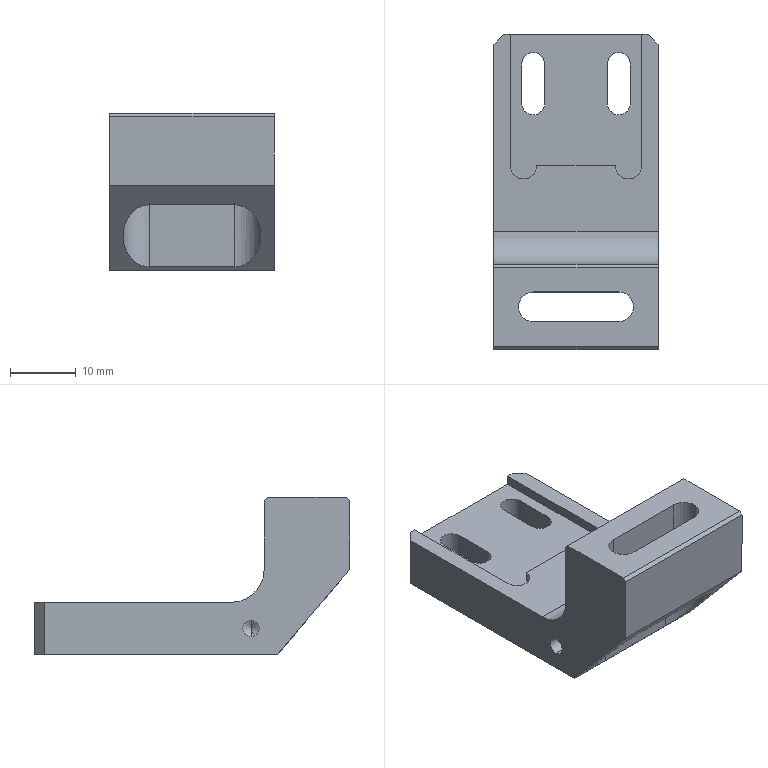Part | SolidWorks | features ICE 4, Cut 3, Chamfer 2, HoleWzd 2, Extrusion 1, Fillet 1, MirrorPattern 1 | 1 solid | 51 faces | box 25 x 48 x 24 mm | volume 9769 mm3 | plane 26 | cylinder 19 | cone 6 | commonest cylinder face diameters 2.5 x6 3.5 x4 4.5 x3 8 x3 4 x2 10 x1
STEP:
#1=CARTESIAN_POINT('',(1.,-9.,1.25));
#2=VERTEX_POINT('',#1);
#3=CARTESIAN_POINT('',(1.,-9.,-1.25));
#4=VERTEX_POINT('',#3);
#5=CARTESIAN_POINT('',(1.,-9.,0.));
#6=DIRECTION('',(1.,0.,0.));
#7=DIRECTION('',(0.,0.,-1.));
#8=AXIS2_PLACEMENT_3D('',#5,#6,#7);
#9=CIRCLE('',#8,1.25);
#10=EDGE_CURVE('',#2,#4,#9,.T.);
#11=ORIENTED_EDGE('',*,*,#10,.F.);
#12=CARTESIAN_POINT('',(12.5,-9.,1.25));
#13=VERTEX_POINT('',#12);
#14=CARTESIAN_POINT('',(12.5,-9.,1.25));
#15=DIRECTION('',(1.,0.,0.));
#16=VECTOR('',#15,1000.);
#17=LINE('',#14,#16);
#18=EDGE_CURVE('',#2,#13,#17,.T.);
#19=ORIENTED_EDGE('',*,*,#18,.T.);
#20=CARTESIAN_POINT('',(12.5,-9.,-1.25));
#21=VERTEX_POINT('',#20);
#22=CARTESIAN_POINT('',(12.5,-9.,0.));
#23=DIRECTION('',(1.,0.,0.));
#24=DIRECTION('',(0.,0.,-1.));
#25=AXIS2_PLACEMENT_3D('',#22,#23,#24);
#26=CIRCLE('',#25,1.25);
#27=EDGE_CURVE('',#13,#21,#26,.T.);
#28=ORIENTED_EDGE('',*,*,#27,.T.);
#29=CARTESIAN_POINT('',(12.5,-9.,-1.25));
#30=DIRECTION('',(1.,0.,0.));
#31=VECTOR('',#30,1000.);
#32=LINE('',#29,#31);
#33=EDGE_CURVE('',#4,#21,#32,.T.);
#34=ORIENTED_EDGE('',*,*,#33,.F.);
#35=EDGE_LOOP('',(#11,#19,#28,#34));
#36=FACE_OUTER_BOUND('',#35,.T.);
#37=CARTESIAN_POINT('',(12.5,-9.,0.));
#38=DIRECTION('',(1.,0.,0.));
#39=DIRECTION('',(0.,0.,-1.));
#40=AXIS2_PLACEMENT_3D('',#37,#38,#39);
#41=CYLINDRICAL_SURFACE('',#40,1.25);
#42=ADVANCED_FACE('',(#36),#41,.F.);
#43=CARTESIAN_POINT('',(0.2489,-9.,0.));
#44=VERTEX_POINT('',#43);
#45=CARTESIAN_POINT('',(1.,-9.,-1.25));
#46=DIRECTION('',(0.515,0.,-0.8572));
#47=VECTOR('',#46,1000.);
#48=LINE('',#45,#47);
#49=EDGE_CURVE('',#44,#4,#48,.T.);
#50=ORIENTED_EDGE('',*,*,#49,.F.);
#51=CARTESIAN_POINT('',(1.,-9.,1.25));
#52=DIRECTION('',(0.515,0.,0.8572));
#53=VECTOR('',#52,1000.);
#54=LINE('',#51,#53);
#55=EDGE_CURVE('',#44,#2,#54,.T.);
#56=ORIENTED_EDGE('',*,*,#55,.T.);
#57=ORIENTED_EDGE('',*,*,#10,.T.);
#58=EDGE_LOOP('',(#50,#56,#57));
#59=FACE_OUTER_BOUND('',#58,.T.);
#60=CARTESIAN_POINT('',(1.,-9.,0.));
#61=DIRECTION('',(1.,0.,0.));
#62=DIRECTION('',(0.,0.,-1.));
#63=AXIS2_PLACEMENT_3D('',#60,#61,#62);
#64=CONICAL_SURFACE('',#63,1.25,1.03);
#65=ADVANCED_FACE('',(#59),#64,.F.);
#66=CARTESIAN_POINT('',(-10.5,-17.5,11.));
#67=VERTEX_POINT('',#66);
#68=CARTESIAN_POINT('',(-6.5,-13.5,11.));
#69=VERTEX_POINT('',#68);
#70=CARTESIAN_POINT('',(-6.5,-17.5,11.));
#71=DIRECTION('',(0.,0.,-1.));
#72=DIRECTION('',(1.,0.,0.));
#73=AXIS2_PLACEMENT_3D('',#70,#71,#72);
#74=CIRCLE('',#73,4.);
#75=EDGE_CURVE('',#67,#69,#74,.T.);
#76=ORIENTED_EDGE('',*,*,#75,.F.);
#77=CARTESIAN_POINT('',(-10.5,-17.5,1.318));
#78=VERTEX_POINT('',#77);
#79=CARTESIAN_POINT('',(-10.5,-17.5,42.472));
#80=DIRECTION('',(0.,0.,-1.));
#81=VECTOR('',#80,1000.);
#82=LINE('',#79,#81);
#83=EDGE_CURVE('',#67,#78,#82,.T.);
#84=ORIENTED_EDGE('',*,*,#83,.T.);
#85=CARTESIAN_POINT('',(-6.5,-13.5,-3.409));
#86=VERTEX_POINT('',#85);
#87=CARTESIAN_POINT('',(-6.5,-13.5,-3.409));
#88=CARTESIAN_POINT('',(-8.843,-13.5,-3.409));
#89=CARTESIAN_POINT('',(-10.5,-15.157,-1.451));
#90=CARTESIAN_POINT('',(-10.5,-17.5,1.318));
#91=(BOUNDED_CURVE()B_SPLINE_CURVE(3,(#87,#88,#89,#90),.UNSPECIFIED.,.F.,.T.)B_SPLINE_CURVE_WITH_KNOTS((4,4),(0.,1.571),.UNSPECIFIED.)CURVE()GEOMETRIC_REPRESENTATION_ITEM()RATIONAL_B_SPLINE_CURVE((1.,0.8047,0.8047,1.))REPRESENTATION_ITEM(''));
#92=EDGE_CURVE('',#86,#78,#91,.T.);
#93=ORIENTED_EDGE('',*,*,#92,.F.);
#94=CARTESIAN_POINT('',(-6.5,-13.5,42.472));
#95=DIRECTION('',(0.,0.,-1.));
#96=VECTOR('',#95,1000.);
#97=LINE('',#94,#96);
#98=EDGE_CURVE('',#69,#86,#97,.T.);
#99=ORIENTED_EDGE('',*,*,#98,.F.);
#100=EDGE_LOOP('',(#76,#84,#93,#99));
#101=FACE_OUTER_BOUND('',#100,.T.);
#102=CARTESIAN_POINT('',(-6.5,-17.5,42.472));
#103=DIRECTION('',(0.,0.,-1.));
#104=DIRECTION('',(-1.,0.,0.));
#105=AXIS2_PLACEMENT_3D('',#102,#103,#104);
#106=CYLINDRICAL_SURFACE('',#105,4.);
#107=ADVANCED_FACE('',(#101),#106,.F.);
#108=CARTESIAN_POINT('',(-8.75,-17.5,20.));
#109=VERTEX_POINT('',#108);
#110=CARTESIAN_POINT('',(-6.5,-15.25,20.));
#111=VERTEX_POINT('',#110);
#112=CARTESIAN_POINT('',(-6.5,-17.5,20.));
#113=DIRECTION('',(0.,0.,-1.));
#114=DIRECTION('',(-1.,0.,0.));
#115=AXIS2_PLACEMENT_3D('',#112,#113,#114);
#116=CIRCLE('',#115,2.25);
#117=EDGE_CURVE('',#109,#111,#116,.T.);
#118=ORIENTED_EDGE('',*,*,#117,.F.);
#119=CARTESIAN_POINT('',(-8.75,-17.5,11.));
#120=VERTEX_POINT('',#119);
#121=CARTESIAN_POINT('',(-8.75,-17.5,20.));
#122=DIRECTION('',(0.,0.,-1.));
#123=VECTOR('',#122,1000.);
#124=LINE('',#121,#123);
#125=EDGE_CURVE('',#109,#120,#124,.T.);
#126=ORIENTED_EDGE('',*,*,#125,.T.);
#127=CARTESIAN_POINT('',(-6.5,-15.25,11.));
#128=VERTEX_POINT('',#127);
#129=CARTESIAN_POINT('',(-6.5,-17.5,11.));
#130=DIRECTION('',(0.,0.,-1.));
#131=DIRECTION('',(1.,0.,0.));
#132=AXIS2_PLACEMENT_3D('',#129,#130,#131);
#133=CIRCLE('',#132,2.25);
#134=EDGE_CURVE('',#120,#128,#133,.T.);
#135=ORIENTED_EDGE('',*,*,#134,.T.);
#136=CARTESIAN_POINT('',(-6.5,-15.25,20.));
#137=DIRECTION('',(0.,0.,-1.));
#138=VECTOR('',#137,1000.);
#139=LINE('',#136,#138);
#140=EDGE_CURVE('',#111,#128,#139,.T.);
#141=ORIENTED_EDGE('',*,*,#140,.F.);
#142=EDGE_LOOP('',(#118,#126,#135,#141));
#143=FACE_OUTER_BOUND('',#142,.T.);
#144=CARTESIAN_POINT('',(-6.5,-17.5,20.));
#145=DIRECTION('',(0.,0.,-1.));
#146=DIRECTION('',(-1.,0.,0.));
#147=AXIS2_PLACEMENT_3D('',#144,#145,#146);
#148=CYLINDRICAL_SURFACE('',#147,2.25);
#149=ADVANCED_FACE('',(#143),#148,.F.);
#150=CARTESIAN_POINT('',(-1.,-9.,-1.25));
#151=VERTEX_POINT('',#150);
#152=CARTESIAN_POINT('',(-1.,-9.,1.25));
#153=VERTEX_POINT('',#152);
#154=CARTESIAN_POINT('',(-1.,-9.,0.));
#155=DIRECTION('',(-1.,0.,0.));
#156=DIRECTION('',(0.,0.,1.));
#157=AXIS2_PLACEMENT_3D('',#154,#155,#156);
#158=CIRCLE('',#157,1.25);
#159=EDGE_CURVE('',#151,#153,#158,.T.);
#160=ORIENTED_EDGE('',*,*,#159,.F.);
#161=CARTESIAN_POINT('',(-12.5,-9.,-1.25));
#162=VERTEX_POINT('',#161);
#163=CARTESIAN_POINT('',(-12.5,-9.,-1.25));
#164=DIRECTION('',(-1.,0.,0.));
#165=VECTOR('',#164,1000.);
#166=LINE('',#163,#165);
#167=EDGE_CURVE('',#151,#162,#166,.T.);
#168=ORIENTED_EDGE('',*,*,#167,.T.);
#169=CARTESIAN_POINT('',(-12.5,-9.,1.25));
#170=VERTEX_POINT('',#169);
#171=CARTESIAN_POINT('',(-12.5,-9.,0.));
#172=DIRECTION('',(-1.,0.,0.));
#173=DIRECTION('',(0.,0.,1.));
#174=AXIS2_PLACEMENT_3D('',#171,#172,#173);
#175=CIRCLE('',#174,1.25);
#176=EDGE_CURVE('',#162,#170,#175,.T.);
#177=ORIENTED_EDGE('',*,*,#176,.T.);
#178=CARTESIAN_POINT('',(-12.5,-9.,1.25));
#179=DIRECTION('',(-1.,0.,0.));
#180=VECTOR('',#179,1000.);
#181=LINE('',#178,#180);
#182=EDGE_CURVE('',#153,#170,#181,.T.);
#183=ORIENTED_EDGE('',*,*,#182,.F.);
#184=EDGE_LOOP('',(#160,#168,#177,#183));
#185=FACE_OUTER_BOUND('',#184,.T.);
#186=CARTESIAN_POINT('',(-12.5,-9.,0.));
#187=DIRECTION('',(-1.,0.,0.));
#188=DIRECTION('',(0.,0.,1.));
#189=AXIS2_PLACEMENT_3D('',#186,#187,#188);
#190=CYLINDRICAL_SURFACE('',#189,1.25);
#191=ADVANCED_FACE('',(#185),#190,.F.);
#192=CARTESIAN_POINT('',(-0.2489,-9.,0.));
#193=VERTEX_POINT('',#192);
#194=CARTESIAN_POINT('',(-1.,-9.,1.25));
#195=DIRECTION('',(-0.515,0.,0.8572));
#196=VECTOR('',#195,1000.);
#197=LINE('',#194,#196);
#198=EDGE_CURVE('',#193,#153,#197,.T.);
#199=ORIENTED_EDGE('',*,*,#198,.F.);
#200=CARTESIAN_POINT('',(-1.,-9.,-1.25));
#201=DIRECTION('',(-0.515,0.,-0.8572));
#202=VECTOR('',#201,1000.);
#203=LINE('',#200,#202);
#204=EDGE_CURVE('',#193,#151,#203,.T.);
#205=ORIENTED_EDGE('',*,*,#204,.T.);
#206=ORIENTED_EDGE('',*,*,#159,.T.);
#207=EDGE_LOOP('',(#199,#205,#206));
#208=FACE_OUTER_BOUND('',#207,.T.);
#209=CARTESIAN_POINT('',(-1.,-9.,0.));
#210=DIRECTION('',(-1.,0.,0.));
#211=DIRECTION('',(0.,0.,1.));
#212=AXIS2_PLACEMENT_3D('',#209,#210,#211);
#213=CONICAL_SURFACE('',#212,1.25,1.03);
#214=ADVANCED_FACE('',(#208),#213,.F.);
#215=CARTESIAN_POINT('',(0.,12.5,-3.25));
#216=VERTEX_POINT('',#215);
#217=CARTESIAN_POINT('',(0.,12.5,-0.75));
#218=VERTEX_POINT('',#217);
#219=CARTESIAN_POINT('',(0.,12.5,-2.));
#220=DIRECTION('',(0.,1.,0.));
#221=DIRECTION('',(0.,0.,1.));
#222=AXIS2_PLACEMENT_3D('',#219,#220,#221);
#223=CIRCLE('',#222,1.25);
#224=EDGE_CURVE('',#216,#218,#223,.T.);
#225=ORIENTED_EDGE('',*,*,#224,.F.);
#226=CARTESIAN_POINT('',(0.,24.,-3.25));
#227=VERTEX_POINT('',#226);
#228=CARTESIAN_POINT('',(0.,24.,-3.25));
#229=DIRECTION('',(0.,1.,0.));
#230=VECTOR('',#229,1000.);
#231=LINE('',#228,#230);
#232=EDGE_CURVE('',#216,#227,#231,.T.);
#233=ORIENTED_EDGE('',*,*,#232,.T.);
#234=CARTESIAN_POINT('',(0.,24.,-0.75));
#235=VERTEX_POINT('',#234);
#236=CARTESIAN_POINT('',(0.,24.,-2.));
#237=DIRECTION('',(0.,1.,0.));
#238=DIRECTION('',(0.,0.,1.));
#239=AXIS2_PLACEMENT_3D('',#236,#237,#238);
#240=CIRCLE('',#239,1.25);
#241=EDGE_CURVE('',#227,#235,#240,.T.);
#242=ORIENTED_EDGE('',*,*,#241,.T.);
#243=CARTESIAN_POINT('',(0.,24.,-0.75));
#244=DIRECTION('',(0.,1.,0.));
#245=VECTOR('',#244,1000.);
#246=LINE('',#243,#245);
#247=EDGE_CURVE('',#218,#235,#246,.T.);
#248=ORIENTED_EDGE('',*,*,#247,.F.);
#249=EDGE_LOOP('',(#225,#233,#242,#248));
#250=FACE_OUTER_BOUND('',#249,.T.);
#251=CARTESIAN_POINT('',(0.,24.,-2.));
#252=DIRECTION('',(0.,1.,0.));
#253=DIRECTION('',(0.,0.,1.));
#254=AXIS2_PLACEMENT_3D('',#251,#252,#253);
#255=CYLINDRICAL_SURFACE('',#254,1.25);
#256=ADVANCED_FACE('',(#250),#255,.F.);
#257=CARTESIAN_POINT('',(0.,11.749,-2.));
#258=VERTEX_POINT('',#257);
#259=CARTESIAN_POINT('',(0.,12.5,-0.75));
#260=DIRECTION('',(0.,0.515,0.8572));
#261=VECTOR('',#260,1000.);
#262=LINE('',#259,#261);
#263=EDGE_CURVE('',#258,#218,#262,.T.);
#264=ORIENTED_EDGE('',*,*,#263,.F.);
#265=CARTESIAN_POINT('',(0.,12.5,-3.25));
#266=DIRECTION('',(0.,0.515,-0.8572));
#267=VECTOR('',#266,1000.);
#268=LINE('',#265,#267);
#269=EDGE_CURVE('',#258,#216,#268,.T.);
#270=ORIENTED_EDGE('',*,*,#269,.T.);
#271=ORIENTED_EDGE('',*,*,#224,.T.);
#272=EDGE_LOOP('',(#264,#270,#271));
#273=FACE_OUTER_BOUND('',#272,.T.);
#274=CARTESIAN_POINT('',(0.,12.5,-2.));
#275=DIRECTION('',(0.,1.,0.));
#276=DIRECTION('',(0.,0.,1.));
#277=AXIS2_PLACEMENT_3D('',#274,#275,#276);
#278=CONICAL_SURFACE('',#277,1.25,1.03);
#279=ADVANCED_FACE('',(#273),#278,.F.);
#280=CARTESIAN_POINT('',(-12.5,22.5,4.));
#281=VERTEX_POINT('',#280);
#282=CARTESIAN_POINT('',(-12.5,-6.,4.));
#283=VERTEX_POINT('',#282);
#284=CARTESIAN_POINT('',(-12.5,-24.,4.));
#285=DIRECTION('',(0.,-1.,0.));
#286=VECTOR('',#285,1000.);
#287=LINE('',#284,#286);
#288=EDGE_CURVE('',#281,#283,#287,.T.);
#289=ORIENTED_EDGE('',*,*,#288,.T.);
#290=CARTESIAN_POINT('',(12.5,-6.,4.));
#291=VERTEX_POINT('',#290);
#292=CARTESIAN_POINT('',(12.5,-6.,4.));
#293=DIRECTION('',(1.,0.,0.));
#294=VECTOR('',#293,1000.);
#295=LINE('',#292,#294);
#296=EDGE_CURVE('',#283,#291,#295,.T.);
#297=ORIENTED_EDGE('',*,*,#296,.T.);
#298=CARTESIAN_POINT('',(12.5,22.5,4.));
#299=VERTEX_POINT('',#298);
#300=CARTESIAN_POINT('',(12.5,-24.,4.));
#301=DIRECTION('',(0.,1.,0.));
#302=VECTOR('',#301,1000.);
#303=LINE('',#300,#302);
#304=EDGE_CURVE('',#291,#299,#303,.T.);
#305=ORIENTED_EDGE('',*,*,#304,.T.);
#306=CARTESIAN_POINT('',(11.,24.,4.));
#307=VERTEX_POINT('',#306);
#308=CARTESIAN_POINT('',(11.,24.,4.));
#309=DIRECTION('',(-0.7071,0.7071,0.));
#310=VECTOR('',#309,1000.);
#311=LINE('',#308,#310);
#312=EDGE_CURVE('',#299,#307,#311,.T.);
#313=ORIENTED_EDGE('',*,*,#312,.T.);
#314=CARTESIAN_POINT('',(10.,24.,4.));
#315=VERTEX_POINT('',#314);
#316=CARTESIAN_POINT('',(-12.5,24.,4.));
#317=DIRECTION('',(-1.,0.,0.));
#318=VECTOR('',#317,1000.);
#319=LINE('',#316,#318);
#320=EDGE_CURVE('',#307,#315,#319,.T.);
#321=ORIENTED_EDGE('',*,*,#320,.T.);
#322=CARTESIAN_POINT('',(10.,4.,4.));
#323=VERTEX_POINT('',#322);
#324=CARTESIAN_POINT('',(10.,4.,4.));
#325=DIRECTION('',(0.,1.,0.));
#326=VECTOR('',#325,1000.);
#327=LINE('',#324,#326);
#328=EDGE_CURVE('',#323,#315,#327,.T.);
#329=ORIENTED_EDGE('',*,*,#328,.F.);
#330=CARTESIAN_POINT('',(6.,4.,4.));
#331=VERTEX_POINT('',#330);
#332=CARTESIAN_POINT('',(8.,4.,4.));
#333=DIRECTION('',(0.,0.,1.));
#334=DIRECTION('',(1.,0.,0.));
#335=AXIS2_PLACEMENT_3D('',#332,#333,#334);
#336=CIRCLE('',#335,2.);
#337=EDGE_CURVE('',#331,#323,#336,.T.);
#338=ORIENTED_EDGE('',*,*,#337,.F.);
#339=CARTESIAN_POINT('',(-6.,4.,4.));
#340=VERTEX_POINT('',#339);
#341=CARTESIAN_POINT('',(-10.,4.,4.));
#342=DIRECTION('',(1.,0.,0.));
#343=VECTOR('',#342,1000.);
#344=LINE('',#341,#343);
#345=EDGE_CURVE('',#340,#331,#344,.T.);
#346=ORIENTED_EDGE('',*,*,#345,.F.);
#347=CARTESIAN_POINT('',(-10.,4.,4.));
#348=VERTEX_POINT('',#347);
#349=CARTESIAN_POINT('',(-8.,4.,4.));
#350=DIRECTION('',(0.,0.,1.));
#351=DIRECTION('',(1.,0.,0.));
#352=AXIS2_PLACEMENT_3D('',#349,#350,#351);
#353=CIRCLE('',#352,2.);
#354=EDGE_CURVE('',#348,#340,#353,.T.);
#355=ORIENTED_EDGE('',*,*,#354,.F.);
#356=CARTESIAN_POINT('',(-10.,24.,4.));
#357=VERTEX_POINT('',#356);
#358=CARTESIAN_POINT('',(-10.,4.,4.));
#359=DIRECTION('',(0.,-1.,0.));
#360=VECTOR('',#359,1000.);
#361=LINE('',#358,#360);
#362=EDGE_CURVE('',#357,#348,#361,.T.);
#363=ORIENTED_EDGE('',*,*,#362,.F.);
#364=CARTESIAN_POINT('',(-11.,24.,4.));
#365=VERTEX_POINT('',#364);
#366=CARTESIAN_POINT('',(-12.5,24.,4.));
#367=DIRECTION('',(-1.,0.,0.));
#368=VECTOR('',#367,1000.);
#369=LINE('',#366,#368);
#370=EDGE_CURVE('',#357,#365,#369,.T.);
#371=ORIENTED_EDGE('',*,*,#370,.T.);
#372=CARTESIAN_POINT('',(-12.5,22.5,4.));
#373=DIRECTION('',(-0.7071,-0.7071,0.));
#374=VECTOR('',#373,1000.);
#375=LINE('',#372,#374);
#376=EDGE_CURVE('',#365,#281,#375,.T.);
#377=ORIENTED_EDGE('',*,*,#376,.T.);
#378=EDGE_LOOP('',(#289,#297,#305,#313,#321,#329,#338,#346,#355,#363,#371,#377));
#379=FACE_OUTER_BOUND('',#378,.T.);
#380=CARTESIAN_POINT('',(0.,0.,4.));
#381=DIRECTION('',(0.,0.,-1.));
#382=DIRECTION('',(-1.,0.,0.));
#383=AXIS2_PLACEMENT_3D('',#380,#381,#382);
#384=PLANE('',#383);
#385=ADVANCED_FACE('',(#379),#384,.F.);
#386=CARTESIAN_POINT('',(12.5,-9.,0.));
#387=DIRECTION('',(1.,0.,0.));
#388=DIRECTION('',(0.,0.,-1.));
#389=AXIS2_PLACEMENT_3D('',#386,#387,#388);
#390=CIRCLE('',#389,1.25);
#391=EDGE_CURVE('',#21,#13,#390,.T.);
#392=ORIENTED_EDGE('',*,*,#391,.F.);
#393=ORIENTED_EDGE('',*,*,#27,.F.);
#394=EDGE_LOOP('',(#392,#393));
#395=FACE_BOUND('',#394,.T.);
#396=CARTESIAN_POINT('',(12.5,-11.5,20.));
#397=VERTEX_POINT('',#396);
#398=CARTESIAN_POINT('',(12.5,-23.5,20.));
#399=VERTEX_POINT('',#398);
#400=CARTESIAN_POINT('',(12.5,-11.,20.));
#401=DIRECTION('',(0.,-1.,0.));
#402=VECTOR('',#401,1000.);
#403=LINE('',#400,#402);
#404=EDGE_CURVE('',#397,#399,#403,.T.);
#405=ORIENTED_EDGE('',*,*,#404,.T.);
#406=CARTESIAN_POINT('',(12.5,-24.,19.5));
#407=VERTEX_POINT('',#406);
#408=CARTESIAN_POINT('',(12.5,-24.,19.5));
#409=DIRECTION('',(0.,-0.7071,-0.7071));
#410=VECTOR('',#409,1000.);
#411=LINE('',#408,#410);
#412=EDGE_CURVE('',#399,#407,#411,.T.);
#413=ORIENTED_EDGE('',*,*,#412,.T.);
#414=CARTESIAN_POINT('',(12.5,-24.,9.));
#415=VERTEX_POINT('',#414);
#416=CARTESIAN_POINT('',(12.5,-24.,4.));
#417=DIRECTION('',(0.,0.,-1.));
#418=VECTOR('',#417,1000.);
#419=LINE('',#416,#418);
#420=EDGE_CURVE('',#407,#415,#419,.T.);
#421=ORIENTED_EDGE('',*,*,#420,.T.);
#422=CARTESIAN_POINT('',(12.5,-13.,-4.));
#423=VERTEX_POINT('',#422);
#424=CARTESIAN_POINT('',(12.5,-24.,9.));
#425=DIRECTION('',(0.,-0.6459,0.7634));
#426=VECTOR('',#425,1000.);
#427=LINE('',#424,#426);
#428=EDGE_CURVE('',#423,#415,#427,.T.);
#429=ORIENTED_EDGE('',*,*,#428,.F.);
#430=CARTESIAN_POINT('',(12.5,22.5,-4.));
#431=VERTEX_POINT('',#430);
#432=CARTESIAN_POINT('',(12.5,-24.,-4.));
#433=DIRECTION('',(0.,1.,0.));
#434=VECTOR('',#433,1000.);
#435=LINE('',#432,#434);
#436=EDGE_CURVE('',#423,#431,#435,.T.);
#437=ORIENTED_EDGE('',*,*,#436,.T.);
#438=CARTESIAN_POINT('',(12.5,22.5,4.));
#439=DIRECTION('',(0.,0.,1.));
#440=VECTOR('',#439,1000.);
#441=LINE('',#438,#440);
#442=EDGE_CURVE('',#431,#299,#441,.T.);
#443=ORIENTED_EDGE('',*,*,#442,.T.);
#444=ORIENTED_EDGE('',*,*,#304,.F.);
#445=CARTESIAN_POINT('',(12.5,-11.,9.));
#446=VERTEX_POINT('',#445);
#447=CARTESIAN_POINT('',(12.5,-6.,9.));
#448=DIRECTION('',(-1.,0.,0.));
#449=DIRECTION('',(0.,0.,1.));
#450=AXIS2_PLACEMENT_3D('',#447,#448,#449);
#451=CIRCLE('',#450,5.);
#452=EDGE_CURVE('',#291,#446,#451,.T.);
#453=ORIENTED_EDGE('',*,*,#452,.T.);
#454=CARTESIAN_POINT('',(12.5,-11.,19.5));
#455=VERTEX_POINT('',#454);
#456=CARTESIAN_POINT('',(12.5,-11.,20.));
#457=DIRECTION('',(0.,0.,1.));
#458=VECTOR('',#457,1000.);
#459=LINE('',#456,#458);
#460=EDGE_CURVE('',#446,#455,#459,.T.);
#461=ORIENTED_EDGE('',*,*,#460,.T.);
#462=CARTESIAN_POINT('',(12.5,-11.5,20.));
#463=DIRECTION('',(0.,-0.7071,0.7071));
#464=VECTOR('',#463,1000.);
#465=LINE('',#462,#464);
#466=EDGE_CURVE('',#455,#397,#465,.T.);
#467=ORIENTED_EDGE('',*,*,#466,.T.);
#468=EDGE_LOOP('',(#405,#413,#421,#429,#437,#443,#444,#453,#461,#467));
#469=FACE_OUTER_BOUND('',#468,.T.);
#470=CARTESIAN_POINT('',(12.5,-24.,4.));
#471=DIRECTION('',(-1.,0.,0.));
#472=DIRECTION('',(0.,0.,1.));
#473=AXIS2_PLACEMENT_3D('',#470,#471,#472);
#474=PLANE('',#473);
#475=ADVANCED_FACE('',(#395,#469),#474,.F.);
#476=CARTESIAN_POINT('',(0.,24.,-2.));
#477=DIRECTION('',(0.,1.,0.));
#478=DIRECTION('',(0.,0.,1.));
#479=AXIS2_PLACEMENT_3D('',#476,#477,#478);
#480=CIRCLE('',#479,1.25);
#481=EDGE_CURVE('',#235,#227,#480,.T.);
#482=ORIENTED_EDGE('',*,*,#481,.F.);
#483=ORIENTED_EDGE('',*,*,#241,.F.);
#484=EDGE_LOOP('',(#482,#483));
#485=FACE_BOUND('',#484,.T.);
#486=ORIENTED_EDGE('',*,*,#320,.F.);
#487=CARTESIAN_POINT('',(11.,24.,-4.));
#488=VERTEX_POINT('',#487);
#489=CARTESIAN_POINT('',(11.,24.,4.));
#490=DIRECTION('',(0.,0.,-1.));
#491=VECTOR('',#490,1000.);
#492=LINE('',#489,#491);
#493=EDGE_CURVE('',#307,#488,#492,.T.);
#494=ORIENTED_EDGE('',*,*,#493,.T.);
#495=CARTESIAN_POINT('',(-11.,24.,-4.));
#496=VERTEX_POINT('',#495);
#497=CARTESIAN_POINT('',(-12.5,24.,-4.));
#498=DIRECTION('',(-1.,0.,0.));
#499=VECTOR('',#498,1000.);
#500=LINE('',#497,#499);
#501=EDGE_CURVE('',#488,#496,#500,.T.);
#502=ORIENTED_EDGE('',*,*,#501,.T.);
#503=CARTESIAN_POINT('',(-11.,24.,4.));
#504=DIRECTION('',(0.,0.,1.));
#505=VECTOR('',#504,1000.);
#506=LINE('',#503,#505);
#507=EDGE_CURVE('',#496,#365,#506,.T.);
#508=ORIENTED_EDGE('',*,*,#507,.T.);
#509=ORIENTED_EDGE('',*,*,#370,.F.);
#510=CARTESIAN_POINT('',(-10.,24.,2.5));
#511=VERTEX_POINT('',#510);
#512=CARTESIAN_POINT('',(-10.,24.,4.));
#513=DIRECTION('',(0.,0.,-1.));
#514=VECTOR('',#513,1000.);
#515=LINE('',#512,#514);
#516=EDGE_CURVE('',#357,#511,#515,.T.);
#517=ORIENTED_EDGE('',*,*,#516,.T.);
#518=CARTESIAN_POINT('',(10.,24.,2.5));
#519=VERTEX_POINT('',#518);
#520=CARTESIAN_POINT('',(-12.5,24.,2.5));
#521=DIRECTION('',(1.,0.,0.));
#522=VECTOR('',#521,1000.);
#523=LINE('',#520,#522);
#524=EDGE_CURVE('',#511,#519,#523,.T.);
#525=ORIENTED_EDGE('',*,*,#524,.T.);
#526=CARTESIAN_POINT('',(10.,24.,4.));
#527=DIRECTION('',(0.,0.,1.));
#528=VECTOR('',#527,1000.);
#529=LINE('',#526,#528);
#530=EDGE_CURVE('',#519,#315,#529,.T.);
#531=ORIENTED_EDGE('',*,*,#530,.T.);
#532=EDGE_LOOP('',(#486,#494,#502,#508,#509,#517,#525,#531));
#533=FACE_OUTER_BOUND('',#532,.T.);
#534=CARTESIAN_POINT('',(-12.5,24.,4.));
#535=DIRECTION('',(0.,-1.,0.));
#536=DIRECTION('',(0.,0.,-1.));
#537=AXIS2_PLACEMENT_3D('',#534,#535,#536);
#538=PLANE('',#537);
#539=ADVANCED_FACE('',(#485,#533),#538,.F.);
#540=CARTESIAN_POINT('',(-12.5,-9.,0.));
#541=DIRECTION('',(-1.,0.,0.));
#542=DIRECTION('',(0.,0.,1.));
#543=AXIS2_PLACEMENT_3D('',#540,#541,#542);
#544=CIRCLE('',#543,1.25);
#545=EDGE_CURVE('',#170,#162,#544,.T.);
#546=ORIENTED_EDGE('',*,*,#545,.F.);
#547=ORIENTED_EDGE('',*,*,#176,.F.);
#548=EDGE_LOOP('',(#546,#547));
#549=FACE_BOUND('',#548,.T.);
#550=CARTESIAN_POINT('',(-12.5,-24.,19.5));
#551=VERTEX_POINT('',#550);
#552=CARTESIAN_POINT('',(-12.5,-24.,9.));
#553=VERTEX_POINT('',#552);
#554=CARTESIAN_POINT('',(-12.5,-24.,4.));
#555=DIRECTION('',(0.,0.,-1.));
#556=VECTOR('',#555,1000.);
#557=LINE('',#554,#556);
#558=EDGE_CURVE('',#551,#553,#557,.T.);
#559=ORIENTED_EDGE('',*,*,#558,.F.);
#560=CARTESIAN_POINT('',(-12.5,-23.5,20.));
#561=VERTEX_POINT('',#560);
#562=CARTESIAN_POINT('',(-12.5,-24.,19.5));
#563=DIRECTION('',(0.,0.7071,0.7071));
#564=VECTOR('',#563,1000.);
#565=LINE('',#562,#564);
#566=EDGE_CURVE('',#551,#561,#565,.T.);
#567=ORIENTED_EDGE('',*,*,#566,.T.);
#568=CARTESIAN_POINT('',(-12.5,-11.5,20.));
#569=VERTEX_POINT('',#568);
#570=CARTESIAN_POINT('',(-12.5,-11.,20.));
#571=DIRECTION('',(0.,-1.,0.));
#572=VECTOR('',#571,1000.);
#573=LINE('',#570,#572);
#574=EDGE_CURVE('',#569,#561,#573,.T.);
#575=ORIENTED_EDGE('',*,*,#574,.F.);
#576=CARTESIAN_POINT('',(-12.5,-11.,19.5));
#577=VERTEX_POINT('',#576);
#578=CARTESIAN_POINT('',(-12.5,-11.5,20.));
#579=DIRECTION('',(0.,0.7071,-0.7071));
#580=VECTOR('',#579,1000.);
#581=LINE('',#578,#580);
#582=EDGE_CURVE('',#569,#577,#581,.T.);
#583=ORIENTED_EDGE('',*,*,#582,.T.);
#584=CARTESIAN_POINT('',(-12.5,-11.,9.));
#585=VERTEX_POINT('',#584);
#586=CARTESIAN_POINT('',(-12.5,-11.,20.));
#587=DIRECTION('',(0.,0.,-1.));
#588=VECTOR('',#587,1000.);
#589=LINE('',#586,#588);
#590=EDGE_CURVE('',#577,#585,#589,.T.);
#591=ORIENTED_EDGE('',*,*,#590,.T.);
#592=CARTESIAN_POINT('',(-12.5,-6.,9.));
#593=DIRECTION('',(1.,0.,0.));
#594=DIRECTION('',(0.,0.,-1.));
#595=AXIS2_PLACEMENT_3D('',#592,#593,#594);
#596=CIRCLE('',#595,5.);
#597=EDGE_CURVE('',#585,#283,#596,.T.);
#598=ORIENTED_EDGE('',*,*,#597,.T.);
#599=ORIENTED_EDGE('',*,*,#288,.F.);
#600=CARTESIAN_POINT('',(-12.5,22.5,-4.));
#601=VERTEX_POINT('',#600);
#602=CARTESIAN_POINT('',(-12.5,22.5,4.));
#603=DIRECTION('',(0.,0.,-1.));
#604=VECTOR('',#603,1000.);
#605=LINE('',#602,#604);
#606=EDGE_CURVE('',#281,#601,#605,.T.);
#607=ORIENTED_EDGE('',*,*,#606,.T.);
#608=CARTESIAN_POINT('',(-12.5,-13.,-4.));
#609=VERTEX_POINT('',#608);
#610=CARTESIAN_POINT('',(-12.5,-24.,-4.));
#611=DIRECTION('',(0.,-1.,0.));
#612=VECTOR('',#611,1000.);
#613=LINE('',#610,#612);
#614=EDGE_CURVE('',#601,#609,#613,.T.);
#615=ORIENTED_EDGE('',*,*,#614,.T.);
#616=CARTESIAN_POINT('',(-12.5,-24.,9.));
#617=DIRECTION('',(0.,-0.6459,0.7634));
#618=VECTOR('',#617,1000.);
#619=LINE('',#616,#618);
#620=EDGE_CURVE('',#609,#553,#619,.T.);
#621=ORIENTED_EDGE('',*,*,#620,.T.);
#622=EDGE_LOOP('',(#559,#567,#575,#583,#591,#598,#599,#607,#615,#621));
#623=FACE_OUTER_BOUND('',#622,.T.);
#624=CARTESIAN_POINT('',(-12.5,-24.,4.));
#625=DIRECTION('',(1.,0.,0.));
#626=DIRECTION('',(0.,0.,-1.));
#627=AXIS2_PLACEMENT_3D('',#624,#625,#626);
#628=PLANE('',#627);
#629=ADVANCED_FACE('',(#549,#623),#628,.F.);
#630=ORIENTED_EDGE('',*,*,#420,.F.);
#631=CARTESIAN_POINT('',(-12.5,-24.,19.5));
#632=DIRECTION('',(-1.,0.,0.));
#633=VECTOR('',#632,1000.);
#634=LINE('',#631,#633);
#635=EDGE_CURVE('',#407,#551,#634,.T.);
#636=ORIENTED_EDGE('',*,*,#635,.T.);
#637=ORIENTED_EDGE('',*,*,#558,.T.);
#638=CARTESIAN_POINT('',(-12.5,-24.,9.));
#639=DIRECTION('',(1.,0.,0.));
#640=VECTOR('',#639,1000.);
#641=LINE('',#638,#640);
#642=EDGE_CURVE('',#553,#415,#641,.T.);
#643=ORIENTED_EDGE('',*,*,#642,.T.);
#644=EDGE_LOOP('',(#630,#636,#637,#643));
#645=FACE_OUTER_BOUND('',#644,.T.);
#646=CARTESIAN_POINT('',(-12.5,-24.,4.));
#647=DIRECTION('',(0.,1.,0.));
#648=DIRECTION('',(0.,0.,1.));
#649=AXIS2_PLACEMENT_3D('',#646,#647,#648);
#650=PLANE('',#649);
#651=ADVANCED_FACE('',(#645),#650,.F.);
#652=CARTESIAN_POINT('',(-12.5,-13.,-4.));
#653=DIRECTION('',(1.,0.,0.));
#654=VECTOR('',#653,1000.);
#655=LINE('',#652,#654);
#656=EDGE_CURVE('',#609,#423,#655,.T.);
#657=ORIENTED_EDGE('',*,*,#656,.F.);
#658=ORIENTED_EDGE('',*,*,#614,.F.);
#659=CARTESIAN_POINT('',(-17.5,17.5,-4.));
#660=DIRECTION('',(0.7071,0.7071,0.));
#661=VECTOR('',#660,1000.);
#662=LINE('',#659,#661);
#663=EDGE_CURVE('',#601,#496,#662,.T.);
#664=ORIENTED_EDGE('',*,*,#663,.T.);
#665=ORIENTED_EDGE('',*,*,#501,.F.);
#666=CARTESIAN_POINT('',(17.5,17.5,-4.));
#667=DIRECTION('',(0.7071,-0.7071,0.));
#668=VECTOR('',#667,1000.);
#669=LINE('',#666,#668);
#670=EDGE_CURVE('',#488,#431,#669,.T.);
#671=ORIENTED_EDGE('',*,*,#670,.T.);
#672=ORIENTED_EDGE('',*,*,#436,.F.);
#673=EDGE_LOOP('',(#657,#658,#664,#665,#671,#672));
#674=FACE_OUTER_BOUND('',#673,.T.);
#675=CARTESIAN_POINT('',(-8.25,19.5,-4.));
#676=VERTEX_POINT('',#675);
#677=CARTESIAN_POINT('',(-4.75,19.5,-4.));
#678=VERTEX_POINT('',#677);
#679=CARTESIAN_POINT('',(-6.5,19.5,-4.));
#680=DIRECTION('',(0.,0.,-1.));
#681=DIRECTION('',(-1.,0.,0.));
#682=AXIS2_PLACEMENT_3D('',#679,#680,#681);
#683=CIRCLE('',#682,1.75);
#684=EDGE_CURVE('',#676,#678,#683,.T.);
#685=ORIENTED_EDGE('',*,*,#684,.F.);
#686=CARTESIAN_POINT('',(-8.25,13.5,-4.));
#687=VERTEX_POINT('',#686);
#688=CARTESIAN_POINT('',(-8.25,19.5,-4.));
#689=DIRECTION('',(0.,1.,0.));
#690=VECTOR('',#689,1000.);
#691=LINE('',#688,#690);
#692=EDGE_CURVE('',#687,#676,#691,.T.);
#693=ORIENTED_EDGE('',*,*,#692,.F.);
#694=CARTESIAN_POINT('',(-4.75,13.5,-4.));
#695=VERTEX_POINT('',#694);
#696=CARTESIAN_POINT('',(-6.5,13.5,-4.));
#697=DIRECTION('',(0.,0.,-1.));
#698=DIRECTION('',(-1.,0.,0.));
#699=AXIS2_PLACEMENT_3D('',#696,#697,#698);
#700=CIRCLE('',#699,1.75);
#701=EDGE_CURVE('',#695,#687,#700,.T.);
#702=ORIENTED_EDGE('',*,*,#701,.F.);
#703=CARTESIAN_POINT('',(-4.75,19.5,-4.));
#704=DIRECTION('',(0.,-1.,0.));
#705=VECTOR('',#704,1000.);
#706=LINE('',#703,#705);
#707=EDGE_CURVE('',#678,#695,#706,.T.);
#708=ORIENTED_EDGE('',*,*,#707,.F.);
#709=EDGE_LOOP('',(#685,#693,#702,#708));
#710=FACE_BOUND('',#709,.T.);
#711=CARTESIAN_POINT('',(4.75,19.5,-4.));
#712=VERTEX_POINT('',#711);
#713=CARTESIAN_POINT('',(8.25,19.5,-4.));
#714=VERTEX_POINT('',#713);
#715=CARTESIAN_POINT('',(6.5,19.5,-4.));
#716=DIRECTION('',(0.,0.,-1.));
#717=DIRECTION('',(-1.,0.,0.));
#718=AXIS2_PLACEMENT_3D('',#715,#716,#717);
#719=CIRCLE('',#718,1.75);
#720=EDGE_CURVE('',#712,#714,#719,.T.);
#721=ORIENTED_EDGE('',*,*,#720,.F.);
#722=CARTESIAN_POINT('',(4.75,13.5,-4.));
#723=VERTEX_POINT('',#722);
#724=CARTESIAN_POINT('',(4.75,19.5,-4.));
#725=DIRECTION('',(0.,1.,0.));
#726=VECTOR('',#725,1000.);
#727=LINE('',#724,#726);
#728=EDGE_CURVE('',#723,#712,#727,.T.);
#729=ORIENTED_EDGE('',*,*,#728,.F.);
#730=CARTESIAN_POINT('',(8.25,13.5,-4.));
#731=VERTEX_POINT('',#730);
#732=CARTESIAN_POINT('',(6.5,13.5,-4.));
#733=DIRECTION('',(0.,0.,-1.));
#734=DIRECTION('',(-1.,0.,0.));
#735=AXIS2_PLACEMENT_3D('',#732,#733,#734);
#736=CIRCLE('',#735,1.75);
#737=EDGE_CURVE('',#731,#723,#736,.T.);
#738=ORIENTED_EDGE('',*,*,#737,.F.);
#739=CARTESIAN_POINT('',(8.25,19.5,-4.));
#740=DIRECTION('',(0.,-1.,0.));
#741=VECTOR('',#740,1000.);
#742=LINE('',#739,#741);
#743=EDGE_CURVE('',#714,#731,#742,.T.);
#744=ORIENTED_EDGE('',*,*,#743,.F.);
#745=EDGE_LOOP('',(#721,#729,#738,#744));
#746=FACE_BOUND('',#745,.T.);
#747=CARTESIAN_POINT('',(0.,0.,-4.));
#748=DIRECTION('',(0.,0.,-1.));
#749=DIRECTION('',(-1.,0.,0.));
#750=AXIS2_PLACEMENT_3D('',#747,#748,#749);
#751=PLANE('',#750);
#752=ADVANCED_FACE('',(#674,#710,#746),#751,.T.);
#753=ORIENTED_EDGE('',*,*,#590,.F.);
#754=CARTESIAN_POINT('',(12.5,-11.,19.5));
#755=DIRECTION('',(1.,0.,0.));
#756=VECTOR('',#755,1000.);
#757=LINE('',#754,#756);
#758=EDGE_CURVE('',#577,#455,#757,.T.);
#759=ORIENTED_EDGE('',*,*,#758,.T.);
#760=ORIENTED_EDGE('',*,*,#460,.F.);
#761=CARTESIAN_POINT('',(-12.5,-11.,9.));
#762=DIRECTION('',(-1.,0.,0.));
#763=VECTOR('',#762,1000.);
#764=LINE('',#761,#763);
#765=EDGE_CURVE('',#446,#585,#764,.T.);
#766=ORIENTED_EDGE('',*,*,#765,.T.);
#767=EDGE_LOOP('',(#753,#759,#760,#766));
#768=FACE_OUTER_BOUND('',#767,.T.);
#769=CARTESIAN_POINT('',(0.,-11.,0.));
#770=DIRECTION('',(0.,-1.,0.));
#771=DIRECTION('',(0.,0.,-1.));
#772=AXIS2_PLACEMENT_3D('',#769,#770,#771);
#773=PLANE('',#772);
#774=ADVANCED_FACE('',(#768),#773,.F.);
#775=CARTESIAN_POINT('',(6.5,-15.25,20.));
#776=VERTEX_POINT('',#775);
#777=CARTESIAN_POINT('',(6.5,-19.75,20.));
#778=VERTEX_POINT('',#777);
#779=CARTESIAN_POINT('',(6.5,-17.5,20.));
#780=DIRECTION('',(0.,0.,-1.));
#781=DIRECTION('',(-1.,0.,0.));
#782=AXIS2_PLACEMENT_3D('',#779,#780,#781);
#783=CIRCLE('',#782,2.25);
#784=EDGE_CURVE('',#776,#778,#783,.T.);
#785=ORIENTED_EDGE('',*,*,#784,.T.);
#786=CARTESIAN_POINT('',(-6.5,-19.75,20.));
#787=VERTEX_POINT('',#786);
#788=CARTESIAN_POINT('',(6.5,-19.75,20.));
#789=DIRECTION('',(-1.,0.,0.));
#790=VECTOR('',#789,1000.);
#791=LINE('',#788,#790);
#792=EDGE_CURVE('',#778,#787,#791,.T.);
#793=ORIENTED_EDGE('',*,*,#792,.T.);
#794=CARTESIAN_POINT('',(-6.5,-17.5,20.));
#795=DIRECTION('',(0.,0.,-1.));
#796=DIRECTION('',(-1.,0.,0.));
#797=AXIS2_PLACEMENT_3D('',#794,#795,#796);
#798=CIRCLE('',#797,2.25);
#799=EDGE_CURVE('',#787,#109,#798,.T.);
#800=ORIENTED_EDGE('',*,*,#799,.T.);
#801=ORIENTED_EDGE('',*,*,#117,.T.);
#802=CARTESIAN_POINT('',(6.5,-15.25,20.));
#803=DIRECTION('',(1.,0.,0.));
#804=VECTOR('',#803,1000.);
#805=LINE('',#802,#804);
#806=EDGE_CURVE('',#111,#776,#805,.T.);
#807=ORIENTED_EDGE('',*,*,#806,.T.);
#808=EDGE_LOOP('',(#785,#793,#800,#801,#807));
#809=FACE_BOUND('',#808,.T.);
#810=ORIENTED_EDGE('',*,*,#574,.T.);
#811=CARTESIAN_POINT('',(12.5,-23.5,20.));
#812=DIRECTION('',(1.,0.,0.));
#813=VECTOR('',#812,1000.);
#814=LINE('',#811,#813);
#815=EDGE_CURVE('',#561,#399,#814,.T.);
#816=ORIENTED_EDGE('',*,*,#815,.T.);
#817=ORIENTED_EDGE('',*,*,#404,.F.);
#818=CARTESIAN_POINT('',(-12.5,-11.5,20.));
#819=DIRECTION('',(-1.,0.,0.));
#820=VECTOR('',#819,1000.);
#821=LINE('',#818,#820);
#822=EDGE_CURVE('',#397,#569,#821,.T.);
#823=ORIENTED_EDGE('',*,*,#822,.T.);
#824=EDGE_LOOP('',(#810,#816,#817,#823));
#825=FACE_OUTER_BOUND('',#824,.T.);
#826=CARTESIAN_POINT('',(-12.5,-11.,20.));
#827=DIRECTION('',(0.,0.,1.));
#828=DIRECTION('',(1.,0.,0.));
#829=AXIS2_PLACEMENT_3D('',#826,#827,#828);
#830=PLANE('',#829);
#831=ADVANCED_FACE('',(#809,#825),#830,.T.);
#832=CARTESIAN_POINT('',(10.,4.,2.5));
#833=VERTEX_POINT('',#832);
#834=CARTESIAN_POINT('',(10.,4.,2.5));
#835=DIRECTION('',(0.,1.,0.));
#836=VECTOR('',#835,1000.);
#837=LINE('',#834,#836);
#838=EDGE_CURVE('',#833,#519,#837,.T.);
#839=ORIENTED_EDGE('',*,*,#838,.F.);
#840=CARTESIAN_POINT('',(10.,4.,2.5));
#841=DIRECTION('',(0.,0.,1.));
#842=VECTOR('',#841,1000.);
#843=LINE('',#840,#842);
#844=EDGE_CURVE('',#833,#323,#843,.T.);
#845=ORIENTED_EDGE('',*,*,#844,.T.);
#846=ORIENTED_EDGE('',*,*,#328,.T.);
#847=ORIENTED_EDGE('',*,*,#530,.F.);
#848=EDGE_LOOP('',(#839,#845,#846,#847));
#849=FACE_OUTER_BOUND('',#848,.T.);
#850=CARTESIAN_POINT('',(10.,4.,2.5));
#851=DIRECTION('',(1.,0.,0.));
#852=DIRECTION('',(0.,0.,-1.));
#853=AXIS2_PLACEMENT_3D('',#850,#851,#852);
#854=PLANE('',#853);
#855=ADVANCED_FACE('',(#849),#854,.F.);
#856=ORIENTED_EDGE('',*,*,#362,.T.);
#857=CARTESIAN_POINT('',(-10.,4.,2.5));
#858=VERTEX_POINT('',#857);
#859=CARTESIAN_POINT('',(-10.,4.,2.5));
#860=DIRECTION('',(0.,0.,1.));
#861=VECTOR('',#860,1000.);
#862=LINE('',#859,#861);
#863=EDGE_CURVE('',#858,#348,#862,.T.);
#864=ORIENTED_EDGE('',*,*,#863,.F.);
#865=CARTESIAN_POINT('',(-10.,4.,2.5));
#866=DIRECTION('',(0.,-1.,0.));
#867=VECTOR('',#866,1000.);
#868=LINE('',#865,#867);
#869=EDGE_CURVE('',#511,#858,#868,.T.);
#870=ORIENTED_EDGE('',*,*,#869,.F.);
#871=ORIENTED_EDGE('',*,*,#516,.F.);
#872=EDGE_LOOP('',(#856,#864,#870,#871));
#873=FACE_OUTER_BOUND('',#872,.T.);
#874=CARTESIAN_POINT('',(-10.,4.,2.5));
#875=DIRECTION('',(-1.,0.,0.));
#876=DIRECTION('',(0.,0.,1.));
#877=AXIS2_PLACEMENT_3D('',#874,#875,#876);
#878=PLANE('',#877);
#879=ADVANCED_FACE('',(#873),#878,.F.);
#880=CARTESIAN_POINT('',(-8.25,13.5,2.5));
#881=VERTEX_POINT('',#880);
#882=CARTESIAN_POINT('',(-8.25,19.5,2.5));
#883=VERTEX_POINT('',#882);
#884=CARTESIAN_POINT('',(-8.25,0.,2.5));
#885=DIRECTION('',(0.,1.,0.));
#886=VECTOR('',#885,1000.);
#887=LINE('',#884,#886);
#888=EDGE_CURVE('',#881,#883,#887,.T.);
#889=ORIENTED_EDGE('',*,*,#888,.T.);
#890=CARTESIAN_POINT('',(-4.75,19.5,2.5));
#891=VERTEX_POINT('',#890);
#892=CARTESIAN_POINT('',(-6.5,19.5,2.5));
#893=DIRECTION('',(0.,0.,-1.));
#894=DIRECTION('',(-1.,0.,0.));
#895=AXIS2_PLACEMENT_3D('',#892,#893,#894);
#896=CIRCLE('',#895,1.75);
#897=EDGE_CURVE('',#883,#891,#896,.T.);
#898=ORIENTED_EDGE('',*,*,#897,.T.);
#899=CARTESIAN_POINT('',(-4.75,13.5,2.5));
#900=VERTEX_POINT('',#899);
#901=CARTESIAN_POINT('',(-4.75,0.,2.5));
#902=DIRECTION('',(0.,-1.,0.));
#903=VECTOR('',#902,1000.);
#904=LINE('',#901,#903);
#905=EDGE_CURVE('',#891,#900,#904,.T.);
#906=ORIENTED_EDGE('',*,*,#905,.T.);
#907=CARTESIAN_POINT('',(-6.5,13.5,2.5));
#908=DIRECTION('',(0.,0.,-1.));
#909=DIRECTION('',(-1.,0.,0.));
#910=AXIS2_PLACEMENT_3D('',#907,#908,#909);
#911=CIRCLE('',#910,1.75);
#912=EDGE_CURVE('',#900,#881,#911,.T.);
#913=ORIENTED_EDGE('',*,*,#912,.T.);
#914=EDGE_LOOP('',(#889,#898,#906,#913));
#915=FACE_BOUND('',#914,.T.);
#916=CARTESIAN_POINT('',(4.75,13.5,2.5));
#917=VERTEX_POINT('',#916);
#918=CARTESIAN_POINT('',(4.75,19.5,2.5));
#919=VERTEX_POINT('',#918);
#920=CARTESIAN_POINT('',(4.75,0.,2.5));
#921=DIRECTION('',(0.,1.,0.));
#922=VECTOR('',#921,1000.);
#923=LINE('',#920,#922);
#924=EDGE_CURVE('',#917,#919,#923,.T.);
#925=ORIENTED_EDGE('',*,*,#924,.T.);
#926=CARTESIAN_POINT('',(8.25,19.5,2.5));
#927=VERTEX_POINT('',#926);
#928=CARTESIAN_POINT('',(6.5,19.5,2.5));
#929=DIRECTION('',(0.,0.,-1.));
#930=DIRECTION('',(-1.,0.,0.));
#931=AXIS2_PLACEMENT_3D('',#928,#929,#930);
#932=CIRCLE('',#931,1.75);
#933=EDGE_CURVE('',#919,#927,#932,.T.);
#934=ORIENTED_EDGE('',*,*,#933,.T.);
#935=CARTESIAN_POINT('',(8.25,13.5,2.5));
#936=VERTEX_POINT('',#935);
#937=CARTESIAN_POINT('',(8.25,0.,2.5));
#938=DIRECTION('',(0.,-1.,0.));
#939=VECTOR('',#938,1000.);
#940=LINE('',#937,#939);
#941=EDGE_CURVE('',#927,#936,#940,.T.);
#942=ORIENTED_EDGE('',*,*,#941,.T.);
#943=CARTESIAN_POINT('',(6.5,13.5,2.5));
#944=DIRECTION('',(0.,0.,-1.));
#945=DIRECTION('',(-1.,0.,0.));
#946=AXIS2_PLACEMENT_3D('',#943,#944,#945);
#947=CIRCLE('',#946,1.75);
#948=EDGE_CURVE('',#936,#917,#947,.T.);
#949=ORIENTED_EDGE('',*,*,#948,.T.);
#950=EDGE_LOOP('',(#925,#934,#942,#949));
#951=FACE_BOUND('',#950,.T.);
#952=CARTESIAN_POINT('',(-6.,4.,2.5));
#953=VERTEX_POINT('',#952);
#954=CARTESIAN_POINT('',(6.,4.,2.5));
#955=VERTEX_POINT('',#954);
#956=CARTESIAN_POINT('',(-10.,4.,2.5));
#957=DIRECTION('',(1.,0.,0.));
#958=VECTOR('',#957,1000.);
#959=LINE('',#956,#958);
#960=EDGE_CURVE('',#953,#955,#959,.T.);
#961=ORIENTED_EDGE('',*,*,#960,.T.);
#962=CARTESIAN_POINT('',(8.,4.,2.5));
#963=DIRECTION('',(0.,0.,1.));
#964=DIRECTION('',(-1.,0.,0.));
#965=AXIS2_PLACEMENT_3D('',#962,#963,#964);
#966=CIRCLE('',#965,2.);
#967=EDGE_CURVE('',#955,#833,#966,.T.);
#968=ORIENTED_EDGE('',*,*,#967,.T.);
#969=ORIENTED_EDGE('',*,*,#838,.T.);
#970=ORIENTED_EDGE('',*,*,#524,.F.);
#971=ORIENTED_EDGE('',*,*,#869,.T.);
#972=CARTESIAN_POINT('',(-8.,4.,2.5));
#973=DIRECTION('',(0.,0.,1.));
#974=DIRECTION('',(-1.,0.,0.));
#975=AXIS2_PLACEMENT_3D('',#972,#973,#974);
#976=CIRCLE('',#975,2.);
#977=EDGE_CURVE('',#858,#953,#976,.T.);
#978=ORIENTED_EDGE('',*,*,#977,.T.);
#979=EDGE_LOOP('',(#961,#968,#969,#970,#971,#978));
#980=FACE_OUTER_BOUND('',#979,.T.);
#981=CARTESIAN_POINT('',(0.,0.,2.5));
#982=DIRECTION('',(0.,0.,-1.));
#983=DIRECTION('',(-1.,0.,0.));
#984=AXIS2_PLACEMENT_3D('',#981,#982,#983);
#985=PLANE('',#984);
#986=ADVANCED_FACE('',(#915,#951,#980),#985,.F.);
#987=ORIENTED_EDGE('',*,*,#345,.T.);
#988=CARTESIAN_POINT('',(6.,4.,-3.157));
#989=DIRECTION('',(0.,0.,-1.));
#990=VECTOR('',#989,1000.);
#991=LINE('',#988,#990);
#992=EDGE_CURVE('',#331,#955,#991,.T.);
#993=ORIENTED_EDGE('',*,*,#992,.T.);
#994=ORIENTED_EDGE('',*,*,#960,.F.);
#995=CARTESIAN_POINT('',(-6.,4.,-3.157));
#996=DIRECTION('',(0.,0.,1.));
#997=VECTOR('',#996,1000.);
#998=LINE('',#995,#997);
#999=EDGE_CURVE('',#953,#340,#998,.T.);
#1000=ORIENTED_EDGE('',*,*,#999,.T.);
#1001=EDGE_LOOP('',(#987,#993,#994,#1000));
#1002=FACE_OUTER_BOUND('',#1001,.T.);
#1003=CARTESIAN_POINT('',(-10.,4.,2.5));
#1004=DIRECTION('',(0.,-1.,0.));
#1005=DIRECTION('',(0.,0.,-1.));
#1006=AXIS2_PLACEMENT_3D('',#1003,#1004,#1005);
#1007=PLANE('',#1006);
#1008=ADVANCED_FACE('',(#1002),#1007,.F.);
#1009=ORIENTED_EDGE('',*,*,#269,.F.);
#1010=ORIENTED_EDGE('',*,*,#263,.T.);
#1011=CARTESIAN_POINT('',(0.,12.5,-2.));
#1012=DIRECTION('',(0.,1.,0.));
#1013=DIRECTION('',(0.,0.,1.));
#1014=AXIS2_PLACEMENT_3D('',#1011,#1012,#1013);
#1015=CIRCLE('',#1014,1.25);
#1016=EDGE_CURVE('',#218,#216,#1015,.T.);
#1017=ORIENTED_EDGE('',*,*,#1016,.T.);
#1018=EDGE_LOOP('',(#1009,#1010,#1017));
#1019=FACE_OUTER_BOUND('',#1018,.T.);
#1020=CARTESIAN_POINT('',(0.,12.5,-2.));
#1021=DIRECTION('',(0.,1.,0.));
#1022=DIRECTION('',(0.,0.,1.));
#1023=AXIS2_PLACEMENT_3D('',#1020,#1021,#1022);
#1024=CONICAL_SURFACE('',#1023,1.25,1.03);
#1025=ADVANCED_FACE('',(#1019),#1024,.F.);
#1026=ORIENTED_EDGE('',*,*,#232,.F.);
#1027=ORIENTED_EDGE('',*,*,#1016,.F.);
#1028=ORIENTED_EDGE('',*,*,#247,.T.);
#1029=ORIENTED_EDGE('',*,*,#481,.T.);
#1030=EDGE_LOOP('',(#1026,#1027,#1028,#1029));
#1031=FACE_OUTER_BOUND('',#1030,.T.);
#1032=CARTESIAN_POINT('',(0.,24.,-2.));
#1033=DIRECTION('',(0.,1.,0.));
#1034=DIRECTION('',(0.,0.,1.));
#1035=AXIS2_PLACEMENT_3D('',#1032,#1033,#1034);
#1036=CYLINDRICAL_SURFACE('',#1035,1.25);
#1037=ADVANCED_FACE('',(#1031),#1036,.F.);
#1038=ORIENTED_EDGE('',*,*,#312,.F.);
#1039=ORIENTED_EDGE('',*,*,#442,.F.);
#1040=ORIENTED_EDGE('',*,*,#670,.F.);
#1041=ORIENTED_EDGE('',*,*,#493,.F.);
#1042=EDGE_LOOP('',(#1038,#1039,#1040,#1041));
#1043=FACE_OUTER_BOUND('',#1042,.T.);
#1044=CARTESIAN_POINT('',(11.,24.,4.));
#1045=DIRECTION('',(-0.7071,-0.7071,0.));
#1046=DIRECTION('',(0.,0.,-1.));
#1047=AXIS2_PLACEMENT_3D('',#1044,#1045,#1046);
#1048=PLANE('',#1047);
#1049=ADVANCED_FACE('',(#1043),#1048,.F.);
#1050=ORIENTED_EDGE('',*,*,#376,.F.);
#1051=ORIENTED_EDGE('',*,*,#507,.F.);
#1052=ORIENTED_EDGE('',*,*,#663,.F.);
#1053=ORIENTED_EDGE('',*,*,#606,.F.);
#1054=EDGE_LOOP('',(#1050,#1051,#1052,#1053));
#1055=FACE_OUTER_BOUND('',#1054,.T.);
#1056=CARTESIAN_POINT('',(-12.5,22.5,4.));
#1057=DIRECTION('',(0.7071,-0.7071,0.));
#1058=DIRECTION('',(0.,0.,-1.));
#1059=AXIS2_PLACEMENT_3D('',#1056,#1057,#1058);
#1060=PLANE('',#1059);
#1061=ADVANCED_FACE('',(#1055),#1060,.F.);
#1062=CARTESIAN_POINT('',(4.75,19.5,20.));
#1063=DIRECTION('',(0.,0.,-1.));
#1064=VECTOR('',#1063,1000.);
#1065=LINE('',#1062,#1064);
#1066=EDGE_CURVE('',#919,#712,#1065,.T.);
#1067=ORIENTED_EDGE('',*,*,#1066,.T.);
#1068=ORIENTED_EDGE('',*,*,#720,.T.);
#1069=CARTESIAN_POINT('',(8.25,19.5,20.));
#1070=DIRECTION('',(0.,0.,-1.));
#1071=VECTOR('',#1070,1000.);
#1072=LINE('',#1069,#1071);
#1073=EDGE_CURVE('',#927,#714,#1072,.T.);
#1074=ORIENTED_EDGE('',*,*,#1073,.F.);
#1075=ORIENTED_EDGE('',*,*,#933,.F.);
#1076=EDGE_LOOP('',(#1067,#1068,#1074,#1075));
#1077=FACE_OUTER_BOUND('',#1076,.T.);
#1078=CARTESIAN_POINT('',(6.5,19.5,20.));
#1079=DIRECTION('',(0.,0.,-1.));
#1080=DIRECTION('',(-1.,0.,0.));
#1081=AXIS2_PLACEMENT_3D('',#1078,#1079,#1080);
#1082=CYLINDRICAL_SURFACE('',#1081,1.75);
#1083=ADVANCED_FACE('',(#1077),#1082,.F.);
#1084=CARTESIAN_POINT('',(4.75,13.5,20.));
#1085=DIRECTION('',(0.,0.,-1.));
#1086=VECTOR('',#1085,1000.);
#1087=LINE('',#1084,#1086);
#1088=EDGE_CURVE('',#917,#723,#1087,.T.);
#1089=ORIENTED_EDGE('',*,*,#1088,.T.);
#1090=ORIENTED_EDGE('',*,*,#728,.T.);
#1091=ORIENTED_EDGE('',*,*,#1066,.F.);
#1092=ORIENTED_EDGE('',*,*,#924,.F.);
#1093=EDGE_LOOP('',(#1089,#1090,#1091,#1092));
#1094=FACE_OUTER_BOUND('',#1093,.T.);
#1095=CARTESIAN_POINT('',(4.75,19.5,20.));
#1096=DIRECTION('',(-1.,0.,0.));
#1097=DIRECTION('',(0.,-1.,0.));
#1098=AXIS2_PLACEMENT_3D('',#1095,#1096,#1097);
#1099=PLANE('',#1098);
#1100=ADVANCED_FACE('',(#1094),#1099,.F.);
#1101=CARTESIAN_POINT('',(8.25,13.5,20.));
#1102=DIRECTION('',(0.,0.,-1.));
#1103=VECTOR('',#1102,1000.);
#1104=LINE('',#1101,#1103);
#1105=EDGE_CURVE('',#936,#731,#1104,.T.);
#1106=ORIENTED_EDGE('',*,*,#1105,.T.);
#1107=ORIENTED_EDGE('',*,*,#737,.T.);
#1108=ORIENTED_EDGE('',*,*,#1088,.F.);
#1109=ORIENTED_EDGE('',*,*,#948,.F.);
#1110=EDGE_LOOP('',(#1106,#1107,#1108,#1109));
#1111=FACE_OUTER_BOUND('',#1110,.T.);
#1112=CARTESIAN_POINT('',(6.5,13.5,20.));
#1113=DIRECTION('',(0.,0.,-1.));
#1114=DIRECTION('',(-1.,0.,0.));
#1115=AXIS2_PLACEMENT_3D('',#1112,#1113,#1114);
#1116=CYLINDRICAL_SURFACE('',#1115,1.75);
#1117=ADVANCED_FACE('',(#1111),#1116,.F.);
#1118=ORIENTED_EDGE('',*,*,#1073,.T.);
#1119=ORIENTED_EDGE('',*,*,#743,.T.);
#1120=ORIENTED_EDGE('',*,*,#1105,.F.);
#1121=ORIENTED_EDGE('',*,*,#941,.F.);
#1122=EDGE_LOOP('',(#1118,#1119,#1120,#1121));
#1123=FACE_OUTER_BOUND('',#1122,.T.);
#1124=CARTESIAN_POINT('',(8.25,19.5,20.));
#1125=DIRECTION('',(1.,0.,0.));
#1126=DIRECTION('',(0.,0.,-1.));
#1127=AXIS2_PLACEMENT_3D('',#1124,#1125,#1126);
#1128=PLANE('',#1127);
#1129=ADVANCED_FACE('',(#1123),#1128,.F.);
#1130=CARTESIAN_POINT('',(-8.25,19.5,20.));
#1131=DIRECTION('',(0.,0.,-1.));
#1132=VECTOR('',#1131,1000.);
#1133=LINE('',#1130,#1132);
#1134=EDGE_CURVE('',#883,#676,#1133,.T.);
#1135=ORIENTED_EDGE('',*,*,#1134,.T.);
#1136=ORIENTED_EDGE('',*,*,#684,.T.);
#1137=CARTESIAN_POINT('',(-4.75,19.5,20.));
#1138=DIRECTION('',(0.,0.,-1.));
#1139=VECTOR('',#1138,1000.);
#1140=LINE('',#1137,#1139);
#1141=EDGE_CURVE('',#891,#678,#1140,.T.);
#1142=ORIENTED_EDGE('',*,*,#1141,.F.);
#1143=ORIENTED_EDGE('',*,*,#897,.F.);
#1144=EDGE_LOOP('',(#1135,#1136,#1142,#1143));
#1145=FACE_OUTER_BOUND('',#1144,.T.);
#1146=CARTESIAN_POINT('',(-6.5,19.5,20.));
#1147=DIRECTION('',(0.,0.,-1.));
#1148=DIRECTION('',(-1.,0.,0.));
#1149=AXIS2_PLACEMENT_3D('',#1146,#1147,#1148);
#1150=CYLINDRICAL_SURFACE('',#1149,1.75);
#1151=ADVANCED_FACE('',(#1145),#1150,.F.);
#1152=CARTESIAN_POINT('',(-8.25,13.5,20.));
#1153=DIRECTION('',(0.,0.,-1.));
#1154=VECTOR('',#1153,1000.);
#1155=LINE('',#1152,#1154);
#1156=EDGE_CURVE('',#881,#687,#1155,.T.);
#1157=ORIENTED_EDGE('',*,*,#1156,.T.);
#1158=ORIENTED_EDGE('',*,*,#692,.T.);
#1159=ORIENTED_EDGE('',*,*,#1134,.F.);
#1160=ORIENTED_EDGE('',*,*,#888,.F.);
#1161=EDGE_LOOP('',(#1157,#1158,#1159,#1160));
#1162=FACE_OUTER_BOUND('',#1161,.T.);
#1163=CARTESIAN_POINT('',(-8.25,19.5,20.));
#1164=DIRECTION('',(-1.,0.,0.));
#1165=DIRECTION('',(0.,-1.,0.));
#1166=AXIS2_PLACEMENT_3D('',#1163,#1164,#1165);
#1167=PLANE('',#1166);
#1168=ADVANCED_FACE('',(#1162),#1167,.F.);
#1169=CARTESIAN_POINT('',(-4.75,13.5,20.));
#1170=DIRECTION('',(0.,0.,-1.));
#1171=VECTOR('',#1170,1000.);
#1172=LINE('',#1169,#1171);
#1173=EDGE_CURVE('',#900,#695,#1172,.T.);
#1174=ORIENTED_EDGE('',*,*,#1173,.T.);
#1175=ORIENTED_EDGE('',*,*,#701,.T.);
#1176=ORIENTED_EDGE('',*,*,#1156,.F.);
#1177=ORIENTED_EDGE('',*,*,#912,.F.);
#1178=EDGE_LOOP('',(#1174,#1175,#1176,#1177));
#1179=FACE_OUTER_BOUND('',#1178,.T.);
#1180=CARTESIAN_POINT('',(-6.5,13.5,20.));
#1181=DIRECTION('',(0.,0.,-1.));
#1182=DIRECTION('',(-1.,0.,0.));
#1183=AXIS2_PLACEMENT_3D('',#1180,#1181,#1182);
#1184=CYLINDRICAL_SURFACE('',#1183,1.75);
#1185=ADVANCED_FACE('',(#1179),#1184,.F.);
#1186=ORIENTED_EDGE('',*,*,#1141,.T.);
#1187=ORIENTED_EDGE('',*,*,#707,.T.);
#1188=ORIENTED_EDGE('',*,*,#1173,.F.);
#1189=ORIENTED_EDGE('',*,*,#905,.F.);
#1190=EDGE_LOOP('',(#1186,#1187,#1188,#1189));
#1191=FACE_OUTER_BOUND('',#1190,.T.);
#1192=CARTESIAN_POINT('',(-4.75,19.5,20.));
#1193=DIRECTION('',(1.,0.,0.));
#1194=DIRECTION('',(0.,0.,-1.));
#1195=AXIS2_PLACEMENT_3D('',#1192,#1193,#1194);
#1196=PLANE('',#1195);
#1197=ADVANCED_FACE('',(#1191),#1196,.F.);
#1198=ORIENTED_EDGE('',*,*,#204,.F.);
#1199=ORIENTED_EDGE('',*,*,#198,.T.);
#1200=CARTESIAN_POINT('',(-1.,-9.,0.));
#1201=DIRECTION('',(-1.,0.,0.));
#1202=DIRECTION('',(0.,0.,1.));
#1203=AXIS2_PLACEMENT_3D('',#1200,#1201,#1202);
#1204=CIRCLE('',#1203,1.25);
#1205=EDGE_CURVE('',#153,#151,#1204,.T.);
#1206=ORIENTED_EDGE('',*,*,#1205,.T.);
#1207=EDGE_LOOP('',(#1198,#1199,#1206));
#1208=FACE_OUTER_BOUND('',#1207,.T.);
#1209=CARTESIAN_POINT('',(-1.,-9.,0.));
#1210=DIRECTION('',(-1.,0.,0.));
#1211=DIRECTION('',(0.,0.,1.));
#1212=AXIS2_PLACEMENT_3D('',#1209,#1210,#1211);
#1213=CONICAL_SURFACE('',#1212,1.25,1.03);
#1214=ADVANCED_FACE('',(#1208),#1213,.F.);
#1215=ORIENTED_EDGE('',*,*,#167,.F.);
#1216=ORIENTED_EDGE('',*,*,#1205,.F.);
#1217=ORIENTED_EDGE('',*,*,#182,.T.);
#1218=ORIENTED_EDGE('',*,*,#545,.T.);
#1219=EDGE_LOOP('',(#1215,#1216,#1217,#1218));
#1220=FACE_OUTER_BOUND('',#1219,.T.);
#1221=CARTESIAN_POINT('',(-12.5,-9.,0.));
#1222=DIRECTION('',(-1.,0.,0.));
#1223=DIRECTION('',(0.,0.,1.));
#1224=AXIS2_PLACEMENT_3D('',#1221,#1222,#1223);
#1225=CYLINDRICAL_SURFACE('',#1224,1.25);
#1226=ADVANCED_FACE('',(#1220),#1225,.F.);
#1227=ORIENTED_EDGE('',*,*,#977,.F.);
#1228=ORIENTED_EDGE('',*,*,#863,.T.);
#1229=ORIENTED_EDGE('',*,*,#354,.T.);
#1230=ORIENTED_EDGE('',*,*,#999,.F.);
#1231=EDGE_LOOP('',(#1227,#1228,#1229,#1230));
#1232=FACE_OUTER_BOUND('',#1231,.T.);
#1233=CARTESIAN_POINT('',(-8.,4.,-3.157));
#1234=DIRECTION('',(0.,0.,1.));
#1235=DIRECTION('',(1.,0.,0.));
#1236=AXIS2_PLACEMENT_3D('',#1233,#1234,#1235);
#1237=CYLINDRICAL_SURFACE('',#1236,2.);
#1238=ADVANCED_FACE('',(#1232),#1237,.F.);
#1239=ORIENTED_EDGE('',*,*,#967,.F.);
#1240=ORIENTED_EDGE('',*,*,#992,.F.);
#1241=ORIENTED_EDGE('',*,*,#337,.T.);
#1242=ORIENTED_EDGE('',*,*,#844,.F.);
#1243=EDGE_LOOP('',(#1239,#1240,#1241,#1242));
#1244=FACE_OUTER_BOUND('',#1243,.T.);
#1245=CARTESIAN_POINT('',(8.,4.,-3.157));
#1246=DIRECTION('',(0.,0.,1.));
#1247=DIRECTION('',(1.,0.,0.));
#1248=AXIS2_PLACEMENT_3D('',#1245,#1246,#1247);
#1249=CYLINDRICAL_SURFACE('',#1248,2.);
#1250=ADVANCED_FACE('',(#1244),#1249,.F.);
#1251=CARTESIAN_POINT('',(6.5,-15.25,11.));
#1252=VERTEX_POINT('',#1251);
#1253=CARTESIAN_POINT('',(6.5,-15.25,20.));
#1254=DIRECTION('',(0.,0.,-1.));
#1255=VECTOR('',#1254,1000.);
#1256=LINE('',#1253,#1255);
#1257=EDGE_CURVE('',#776,#1252,#1256,.T.);
#1258=ORIENTED_EDGE('',*,*,#1257,.T.);
#1259=CARTESIAN_POINT('',(6.5,-19.75,11.));
#1260=VERTEX_POINT('',#1259);
#1261=CARTESIAN_POINT('',(6.5,-17.5,11.));
#1262=DIRECTION('',(0.,0.,-1.));
#1263=DIRECTION('',(1.,0.,0.));
#1264=AXIS2_PLACEMENT_3D('',#1261,#1262,#1263);
#1265=CIRCLE('',#1264,2.25);
#1266=EDGE_CURVE('',#1252,#1260,#1265,.T.);
#1267=ORIENTED_EDGE('',*,*,#1266,.T.);
#1268=CARTESIAN_POINT('',(6.5,-19.75,20.));
#1269=DIRECTION('',(0.,0.,-1.));
#1270=VECTOR('',#1269,1000.);
#1271=LINE('',#1268,#1270);
#1272=EDGE_CURVE('',#778,#1260,#1271,.T.);
#1273=ORIENTED_EDGE('',*,*,#1272,.F.);
#1274=ORIENTED_EDGE('',*,*,#784,.F.);
#1275=EDGE_LOOP('',(#1258,#1267,#1273,#1274));
#1276=FACE_OUTER_BOUND('',#1275,.T.);
#1277=CARTESIAN_POINT('',(6.5,-17.5,20.));
#1278=DIRECTION('',(0.,0.,-1.));
#1279=DIRECTION('',(-1.,0.,0.));
#1280=AXIS2_PLACEMENT_3D('',#1277,#1278,#1279);
#1281=CYLINDRICAL_SURFACE('',#1280,2.25);
#1282=ADVANCED_FACE('',(#1276),#1281,.F.);
#1283=ORIENTED_EDGE('',*,*,#140,.T.);
#1284=CARTESIAN_POINT('',(6.5,-15.25,11.));
#1285=DIRECTION('',(1.,0.,0.));
#1286=VECTOR('',#1285,1000.);
#1287=LINE('',#1284,#1286);
#1288=EDGE_CURVE('',#128,#1252,#1287,.T.);
#1289=ORIENTED_EDGE('',*,*,#1288,.T.);
#1290=ORIENTED_EDGE('',*,*,#1257,.F.);
#1291=ORIENTED_EDGE('',*,*,#806,.F.);
#1292=EDGE_LOOP('',(#1283,#1289,#1290,#1291));
#1293=FACE_OUTER_BOUND('',#1292,.T.);
#1294=CARTESIAN_POINT('',(6.5,-15.25,20.));
#1295=DIRECTION('',(0.,1.,0.));
#1296=DIRECTION('',(0.,0.,1.));
#1297=AXIS2_PLACEMENT_3D('',#1294,#1295,#1296);
#1298=PLANE('',#1297);
#1299=ADVANCED_FACE('',(#1293),#1298,.F.);
#1300=ORIENTED_EDGE('',*,*,#125,.F.);
#1301=ORIENTED_EDGE('',*,*,#799,.F.);
#1302=CARTESIAN_POINT('',(-6.5,-19.75,11.));
#1303=VERTEX_POINT('',#1302);
#1304=CARTESIAN_POINT('',(-6.5,-19.75,20.));
#1305=DIRECTION('',(0.,0.,-1.));
#1306=VECTOR('',#1305,1000.);
#1307=LINE('',#1304,#1306);
#1308=EDGE_CURVE('',#787,#1303,#1307,.T.);
#1309=ORIENTED_EDGE('',*,*,#1308,.T.);
#1310=CARTESIAN_POINT('',(-6.5,-17.5,11.));
#1311=DIRECTION('',(0.,0.,-1.));
#1312=DIRECTION('',(1.,0.,0.));
#1313=AXIS2_PLACEMENT_3D('',#1310,#1311,#1312);
#1314=CIRCLE('',#1313,2.25);
#1315=EDGE_CURVE('',#1303,#120,#1314,.T.);
#1316=ORIENTED_EDGE('',*,*,#1315,.T.);
#1317=EDGE_LOOP('',(#1300,#1301,#1309,#1316));
#1318=FACE_OUTER_BOUND('',#1317,.T.);
#1319=CARTESIAN_POINT('',(-6.5,-17.5,20.));
#1320=DIRECTION('',(0.,0.,-1.));
#1321=DIRECTION('',(-1.,0.,0.));
#1322=AXIS2_PLACEMENT_3D('',#1319,#1320,#1321);
#1323=CYLINDRICAL_SURFACE('',#1322,2.25);
#1324=ADVANCED_FACE('',(#1318),#1323,.F.);
#1325=ORIENTED_EDGE('',*,*,#1272,.T.);
#1326=CARTESIAN_POINT('',(6.5,-19.75,11.));
#1327=DIRECTION('',(-1.,0.,0.));
#1328=VECTOR('',#1327,1000.);
#1329=LINE('',#1326,#1328);
#1330=EDGE_CURVE('',#1260,#1303,#1329,.T.);
#1331=ORIENTED_EDGE('',*,*,#1330,.T.);
#1332=ORIENTED_EDGE('',*,*,#1308,.F.);
#1333=ORIENTED_EDGE('',*,*,#792,.F.);
#1334=EDGE_LOOP('',(#1325,#1331,#1332,#1333));
#1335=FACE_OUTER_BOUND('',#1334,.T.);
#1336=CARTESIAN_POINT('',(6.5,-19.75,20.));
#1337=DIRECTION('',(0.,-1.,0.));
#1338=DIRECTION('',(0.,0.,-1.));
#1339=AXIS2_PLACEMENT_3D('',#1336,#1337,#1338);
#1340=PLANE('',#1339);
#1341=ADVANCED_FACE('',(#1335),#1340,.F.);
#1342=ORIENTED_EDGE('',*,*,#92,.T.);
#1343=CARTESIAN_POINT('',(-6.5,-21.5,6.045));
#1344=VERTEX_POINT('',#1343);
#1345=CARTESIAN_POINT('',(-10.5,-17.5,1.318));
#1346=CARTESIAN_POINT('',(-10.5,-19.843,4.087));
#1347=CARTESIAN_POINT('',(-8.843,-21.5,6.045));
#1348=CARTESIAN_POINT('',(-6.5,-21.5,6.045));
#1349=(BOUNDED_CURVE()B_SPLINE_CURVE(3,(#1345,#1346,#1347,#1348),.UNSPECIFIED.,.F.,.T.)B_SPLINE_CURVE_WITH_KNOTS((4,4),(1.571,3.142),.UNSPECIFIED.)CURVE()GEOMETRIC_REPRESENTATION_ITEM()RATIONAL_B_SPLINE_CURVE((1.,0.8047,0.8047,1.))REPRESENTATION_ITEM(''));
#1350=EDGE_CURVE('',#78,#1344,#1349,.T.);
#1351=ORIENTED_EDGE('',*,*,#1350,.T.);
#1352=CARTESIAN_POINT('',(6.5,-21.5,6.045));
#1353=VERTEX_POINT('',#1352);
#1354=CARTESIAN_POINT('',(-12.5,-21.5,6.045));
#1355=DIRECTION('',(1.,0.,0.));
#1356=VECTOR('',#1355,1000.);
#1357=LINE('',#1354,#1356);
#1358=EDGE_CURVE('',#1344,#1353,#1357,.T.);
#1359=ORIENTED_EDGE('',*,*,#1358,.T.);
#1360=CARTESIAN_POINT('',(6.5,-13.5,-3.409));
#1361=VERTEX_POINT('',#1360);
#1362=CARTESIAN_POINT('',(6.5,-21.5,6.045));
#1363=CARTESIAN_POINT('',(14.5,-21.5,6.045));
#1364=CARTESIAN_POINT('',(14.5,-13.5,-3.409));
#1365=CARTESIAN_POINT('',(6.5,-13.5,-3.409));
#1366=(BOUNDED_CURVE()B_SPLINE_CURVE(3,(#1362,#1363,#1364,#1365),.UNSPECIFIED.,.F.,.T.)B_SPLINE_CURVE_WITH_KNOTS((4,4),(3.142,6.283),.UNSPECIFIED.)CURVE()GEOMETRIC_REPRESENTATION_ITEM()RATIONAL_B_SPLINE_CURVE((1.,0.3333,0.3333,1.))REPRESENTATION_ITEM(''));
#1367=EDGE_CURVE('',#1353,#1361,#1366,.T.);
#1368=ORIENTED_EDGE('',*,*,#1367,.T.);
#1369=CARTESIAN_POINT('',(-12.5,-13.5,-3.409));
#1370=DIRECTION('',(-1.,0.,0.));
#1371=VECTOR('',#1370,1000.);
#1372=LINE('',#1369,#1371);
#1373=EDGE_CURVE('',#1361,#86,#1372,.T.);
#1374=ORIENTED_EDGE('',*,*,#1373,.T.);
#1375=EDGE_LOOP('',(#1342,#1351,#1359,#1368,#1374));
#1376=FACE_BOUND('',#1375,.T.);
#1377=ORIENTED_EDGE('',*,*,#428,.T.);
#1378=ORIENTED_EDGE('',*,*,#642,.F.);
#1379=ORIENTED_EDGE('',*,*,#620,.F.);
#1380=ORIENTED_EDGE('',*,*,#656,.T.);
#1381=EDGE_LOOP('',(#1377,#1378,#1379,#1380));
#1382=FACE_OUTER_BOUND('',#1381,.T.);
#1383=CARTESIAN_POINT('',(-12.5,-24.,9.));
#1384=DIRECTION('',(0.,0.7634,0.6459));
#1385=DIRECTION('',(0.,-0.6459,0.7634));
#1386=AXIS2_PLACEMENT_3D('',#1383,#1384,#1385);
#1387=PLANE('',#1386);
#1388=ADVANCED_FACE('',(#1376,#1382),#1387,.F.);
#1389=CARTESIAN_POINT('',(6.5,-13.5,11.));
#1390=VERTEX_POINT('',#1389);
#1391=CARTESIAN_POINT('',(6.5,-21.5,11.));
#1392=VERTEX_POINT('',#1391);
#1393=CARTESIAN_POINT('',(6.5,-17.5,11.));
#1394=DIRECTION('',(0.,0.,-1.));
#1395=DIRECTION('',(1.,0.,0.));
#1396=AXIS2_PLACEMENT_3D('',#1393,#1394,#1395);
#1397=CIRCLE('',#1396,4.);
#1398=EDGE_CURVE('',#1390,#1392,#1397,.T.);
#1399=ORIENTED_EDGE('',*,*,#1398,.T.);
#1400=CARTESIAN_POINT('',(-6.5,-21.5,11.));
#1401=VERTEX_POINT('',#1400);
#1402=CARTESIAN_POINT('',(6.5,-21.5,11.));
#1403=DIRECTION('',(-1.,0.,0.));
#1404=VECTOR('',#1403,1000.);
#1405=LINE('',#1402,#1404);
#1406=EDGE_CURVE('',#1392,#1401,#1405,.T.);
#1407=ORIENTED_EDGE('',*,*,#1406,.T.);
#1408=CARTESIAN_POINT('',(-6.5,-17.5,11.));
#1409=DIRECTION('',(0.,0.,-1.));
#1410=DIRECTION('',(1.,0.,0.));
#1411=AXIS2_PLACEMENT_3D('',#1408,#1409,#1410);
#1412=CIRCLE('',#1411,4.);
#1413=EDGE_CURVE('',#1401,#67,#1412,.T.);
#1414=ORIENTED_EDGE('',*,*,#1413,.T.);
#1415=ORIENTED_EDGE('',*,*,#75,.T.);
#1416=CARTESIAN_POINT('',(6.5,-13.5,11.));
#1417=DIRECTION('',(1.,0.,0.));
#1418=VECTOR('',#1417,1000.);
#1419=LINE('',#1416,#1418);
#1420=EDGE_CURVE('',#69,#1390,#1419,.T.);
#1421=ORIENTED_EDGE('',*,*,#1420,.T.);
#1422=EDGE_LOOP('',(#1399,#1407,#1414,#1415,#1421));
#1423=FACE_OUTER_BOUND('',#1422,.T.);
#1424=ORIENTED_EDGE('',*,*,#1288,.F.);
#1425=ORIENTED_EDGE('',*,*,#134,.F.);
#1426=ORIENTED_EDGE('',*,*,#1315,.F.);
#1427=ORIENTED_EDGE('',*,*,#1330,.F.);
#1428=ORIENTED_EDGE('',*,*,#1266,.F.);
#1429=EDGE_LOOP('',(#1424,#1425,#1426,#1427,#1428));
#1430=FACE_BOUND('',#1429,.T.);
#1431=CARTESIAN_POINT('',(-12.5,-11.,11.));
#1432=DIRECTION('',(0.,0.,1.));
#1433=DIRECTION('',(1.,0.,0.));
#1434=AXIS2_PLACEMENT_3D('',#1431,#1432,#1433);
#1435=PLANE('',#1434);
#1436=ADVANCED_FACE('',(#1423,#1430),#1435,.F.);
#1437=CARTESIAN_POINT('',(-6.5,-21.5,42.472));
#1438=DIRECTION('',(0.,0.,-1.));
#1439=VECTOR('',#1438,1000.);
#1440=LINE('',#1437,#1439);
#1441=EDGE_CURVE('',#1401,#1344,#1440,.T.);
#1442=ORIENTED_EDGE('',*,*,#1441,.F.);
#1443=ORIENTED_EDGE('',*,*,#1406,.F.);
#1444=CARTESIAN_POINT('',(6.5,-21.5,42.472));
#1445=DIRECTION('',(0.,0.,-1.));
#1446=VECTOR('',#1445,1000.);
#1447=LINE('',#1444,#1446);
#1448=EDGE_CURVE('',#1392,#1353,#1447,.T.);
#1449=ORIENTED_EDGE('',*,*,#1448,.T.);
#1450=ORIENTED_EDGE('',*,*,#1358,.F.);
#1451=EDGE_LOOP('',(#1442,#1443,#1449,#1450));
#1452=FACE_OUTER_BOUND('',#1451,.T.);
#1453=CARTESIAN_POINT('',(6.5,-21.5,42.472));
#1454=DIRECTION('',(0.,-1.,0.));
#1455=DIRECTION('',(0.,0.,-1.));
#1456=AXIS2_PLACEMENT_3D('',#1453,#1454,#1455);
#1457=PLANE('',#1456);
#1458=ADVANCED_FACE('',(#1452),#1457,.F.);
#1459=ORIENTED_EDGE('',*,*,#83,.F.);
#1460=ORIENTED_EDGE('',*,*,#1413,.F.);
#1461=ORIENTED_EDGE('',*,*,#1441,.T.);
#1462=ORIENTED_EDGE('',*,*,#1350,.F.);
#1463=EDGE_LOOP('',(#1459,#1460,#1461,#1462));
#1464=FACE_OUTER_BOUND('',#1463,.T.);
#1465=CARTESIAN_POINT('',(-6.5,-17.5,42.472));
#1466=DIRECTION('',(0.,0.,-1.));
#1467=DIRECTION('',(-1.,0.,0.));
#1468=AXIS2_PLACEMENT_3D('',#1465,#1466,#1467);
#1469=CYLINDRICAL_SURFACE('',#1468,4.);
#1470=ADVANCED_FACE('',(#1464),#1469,.F.);
#1471=CARTESIAN_POINT('',(6.5,-13.5,42.472));
#1472=DIRECTION('',(0.,0.,-1.));
#1473=VECTOR('',#1472,1000.);
#1474=LINE('',#1471,#1473);
#1475=EDGE_CURVE('',#1390,#1361,#1474,.T.);
#1476=ORIENTED_EDGE('',*,*,#1475,.F.);
#1477=ORIENTED_EDGE('',*,*,#1420,.F.);
#1478=ORIENTED_EDGE('',*,*,#98,.T.);
#1479=ORIENTED_EDGE('',*,*,#1373,.F.);
#1480=EDGE_LOOP('',(#1476,#1477,#1478,#1479));
#1481=FACE_OUTER_BOUND('',#1480,.T.);
#1482=CARTESIAN_POINT('',(6.5,-13.5,42.472));
#1483=DIRECTION('',(0.,1.,0.));
#1484=DIRECTION('',(0.,0.,1.));
#1485=AXIS2_PLACEMENT_3D('',#1482,#1483,#1484);
#1486=PLANE('',#1485);
#1487=ADVANCED_FACE('',(#1481),#1486,.F.);
#1488=ORIENTED_EDGE('',*,*,#1448,.F.);
#1489=ORIENTED_EDGE('',*,*,#1398,.F.);
#1490=ORIENTED_EDGE('',*,*,#1475,.T.);
#1491=ORIENTED_EDGE('',*,*,#1367,.F.);
#1492=EDGE_LOOP('',(#1488,#1489,#1490,#1491));
#1493=FACE_OUTER_BOUND('',#1492,.T.);
#1494=CARTESIAN_POINT('',(6.5,-17.5,42.472));
#1495=DIRECTION('',(0.,0.,-1.));
#1496=DIRECTION('',(-1.,0.,0.));
#1497=AXIS2_PLACEMENT_3D('',#1494,#1495,#1496);
#1498=CYLINDRICAL_SURFACE('',#1497,4.);
#1499=ADVANCED_FACE('',(#1493),#1498,.F.);
#1500=ORIENTED_EDGE('',*,*,#452,.F.);
#1501=ORIENTED_EDGE('',*,*,#296,.F.);
#1502=ORIENTED_EDGE('',*,*,#597,.F.);
#1503=ORIENTED_EDGE('',*,*,#765,.F.);
#1504=EDGE_LOOP('',(#1500,#1501,#1502,#1503));
#1505=FACE_OUTER_BOUND('',#1504,.T.);
#1506=CARTESIAN_POINT('',(0.,-6.,9.));
#1507=DIRECTION('',(1.,0.,0.));
#1508=DIRECTION('',(0.,0.,-1.));
#1509=AXIS2_PLACEMENT_3D('',#1506,#1507,#1508);
#1510=CYLINDRICAL_SURFACE('',#1509,5.);
#1511=ADVANCED_FACE('',(#1505),#1510,.F.);
#1512=ORIENTED_EDGE('',*,*,#55,.F.);
#1513=ORIENTED_EDGE('',*,*,#49,.T.);
#1514=CARTESIAN_POINT('',(1.,-9.,0.));
#1515=DIRECTION('',(1.,0.,0.));
#1516=DIRECTION('',(0.,0.,-1.));
#1517=AXIS2_PLACEMENT_3D('',#1514,#1515,#1516);
#1518=CIRCLE('',#1517,1.25);
#1519=EDGE_CURVE('',#4,#2,#1518,.T.);
#1520=ORIENTED_EDGE('',*,*,#1519,.T.);
#1521=EDGE_LOOP('',(#1512,#1513,#1520));
#1522=FACE_OUTER_BOUND('',#1521,.T.);
#1523=CARTESIAN_POINT('',(1.,-9.,0.));
#1524=DIRECTION('',(1.,0.,0.));
#1525=DIRECTION('',(0.,0.,-1.));
#1526=AXIS2_PLACEMENT_3D('',#1523,#1524,#1525);
#1527=CONICAL_SURFACE('',#1526,1.25,1.03);
#1528=ADVANCED_FACE('',(#1522),#1527,.F.);
#1529=ORIENTED_EDGE('',*,*,#18,.F.);
#1530=ORIENTED_EDGE('',*,*,#1519,.F.);
#1531=ORIENTED_EDGE('',*,*,#33,.T.);
#1532=ORIENTED_EDGE('',*,*,#391,.T.);
#1533=EDGE_LOOP('',(#1529,#1530,#1531,#1532));
#1534=FACE_OUTER_BOUND('',#1533,.T.);
#1535=CARTESIAN_POINT('',(12.5,-9.,0.));
#1536=DIRECTION('',(1.,0.,0.));
#1537=DIRECTION('',(0.,0.,-1.));
#1538=AXIS2_PLACEMENT_3D('',#1535,#1536,#1537);
#1539=CYLINDRICAL_SURFACE('',#1538,1.25);
#1540=ADVANCED_FACE('',(#1534),#1539,.F.);
#1541=ORIENTED_EDGE('',*,*,#412,.F.);
#1542=ORIENTED_EDGE('',*,*,#815,.F.);
#1543=ORIENTED_EDGE('',*,*,#566,.F.);
#1544=ORIENTED_EDGE('',*,*,#635,.F.);
#1545=EDGE_LOOP('',(#1541,#1542,#1543,#1544));
#1546=FACE_OUTER_BOUND('',#1545,.T.);
#1547=CARTESIAN_POINT('',(-12.5,-24.,19.5));
#1548=DIRECTION('',(0.,-0.7071,0.7071));
#1549=DIRECTION('',(1.,0.,0.));
#1550=AXIS2_PLACEMENT_3D('',#1547,#1548,#1549);
#1551=PLANE('',#1550);
#1552=ADVANCED_FACE('',(#1546),#1551,.T.);
#1553=ORIENTED_EDGE('',*,*,#466,.F.);
#1554=ORIENTED_EDGE('',*,*,#758,.F.);
#1555=ORIENTED_EDGE('',*,*,#582,.F.);
#1556=ORIENTED_EDGE('',*,*,#822,.F.);
#1557=EDGE_LOOP('',(#1553,#1554,#1555,#1556));
#1558=FACE_OUTER_BOUND('',#1557,.T.);
#1559=CARTESIAN_POINT('',(-12.5,-11.5,20.));
#1560=DIRECTION('',(0.,0.7071,0.7071));
#1561=DIRECTION('',(1.,0.,0.));
#1562=AXIS2_PLACEMENT_3D('',#1559,#1560,#1561);
#1563=PLANE('',#1562);
#1564=ADVANCED_FACE('',(#1558),#1563,.T.);
#1565=CLOSED_SHELL('',(#42,#65,#107,#149,#191,#214,#256,#279,#385,#475,#539,#629,#651,#752,#774,#831,#855,#879,#986,#1008,#1025,#1037,#1049,#1061,#1083,#1100,#1117,#1129,#1151,#1168,#1185,#1197,#1214,#1226,#1238,#1250,#1282,#1299,#1324,#1341,#1388,#1436,#1458,#1470,#1487,#1499,#1511,#1528,#1540,#1552,#1564));
#1566=MANIFOLD_SOLID_BREP('',#1565);
#1567=CARTESIAN_POINT('',(0.,0.,0.));
#1568=DIRECTION('',(0.,0.,1.));
#1569=DIRECTION('',(1.,0.,0.));
#1570=AXIS2_PLACEMENT_3D('',#1567,#1568,#1569);
#1571=(LENGTH_UNIT()NAMED_UNIT(*)SI_UNIT(.MILLI.,.METRE.));
#1572=UNCERTAINTY_MEASURE_WITH_UNIT(LENGTH_MEASURE(0.00001),#1571,'','');
#1573=(NAMED_UNIT(*)PLANE_ANGLE_UNIT()SI_UNIT($,.RADIAN.));
#1574=(NAMED_UNIT(*)SI_UNIT($,.STERADIAN.)SOLID_ANGLE_UNIT());
#1575=(GEOMETRIC_REPRESENTATION_CONTEXT(3)GLOBAL_UNCERTAINTY_ASSIGNED_CONTEXT((#1572))GLOBAL_UNIT_ASSIGNED_CONTEXT((#1571,#1573,#1574))REPRESENTATION_CONTEXT('',''));
#1576=ADVANCED_BREP_SHAPE_REPRESENTATION('',(#1566,#1570),#1575);